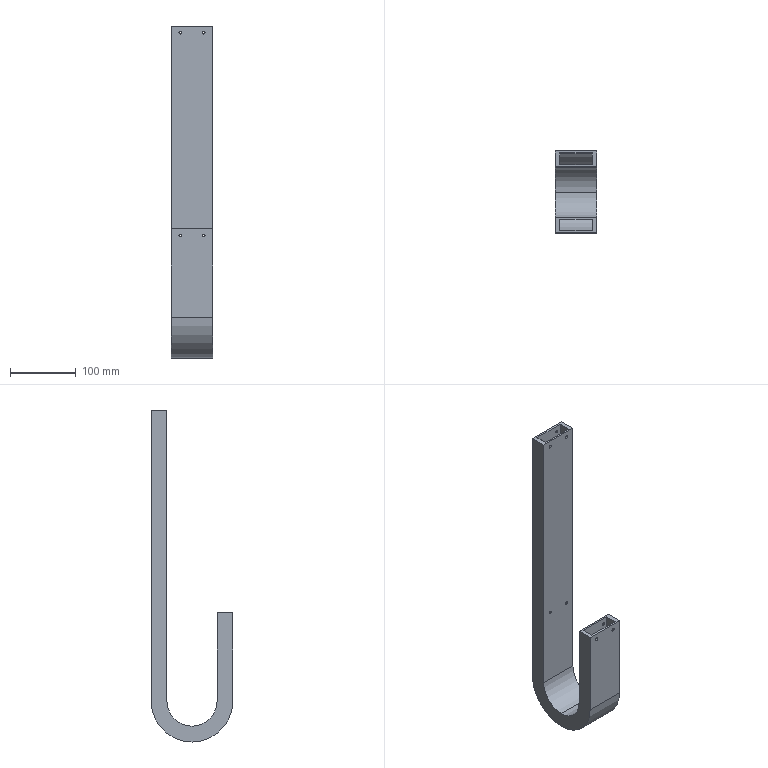Part | SolidWorks | features ICE 1, Sweep 1 | 1 solid | 46 faces | box 63 x 124 x 504 mm | volume 448072 mm3 | cylinder 32 | plane 14 | commonest cylinder face diameters 4.5 x24 76 x2 82 x2 118 x2 124 x2
STEP:
#1=CARTESIAN_POINT('',(15.25,112.,298.));
#2=VERTEX_POINT('',#1);
#3=CARTESIAN_POINT('',(19.75,112.,298.));
#4=VERTEX_POINT('',#3);
#5=CARTESIAN_POINT('',(17.5,112.,298.));
#6=DIRECTION('',(0.,-1.,0.));
#7=DIRECTION('',(1.,0.,0.));
#8=AXIS2_PLACEMENT_3D('',#5,#6,#7);
#9=CIRCLE('',#8,2.25);
#10=EDGE_CURVE('',#2,#4,#9,.T.);
#11=ORIENTED_EDGE('',*,*,#10,.F.);
#12=CARTESIAN_POINT('',(15.25,109.,298.));
#13=VERTEX_POINT('',#12);
#14=CARTESIAN_POINT('',(15.25,112.,298.));
#15=DIRECTION('',(0.,-1.,0.));
#16=VECTOR('',#15,1000.);
#17=LINE('',#14,#16);
#18=EDGE_CURVE('',#2,#13,#17,.T.);
#19=ORIENTED_EDGE('',*,*,#18,.T.);
#20=CARTESIAN_POINT('',(19.75,109.,298.));
#21=VERTEX_POINT('',#20);
#22=CARTESIAN_POINT('',(17.5,109.,298.));
#23=DIRECTION('',(0.,-1.,0.));
#24=DIRECTION('',(1.,0.,0.));
#25=AXIS2_PLACEMENT_3D('',#22,#23,#24);
#26=CIRCLE('',#25,2.25);
#27=EDGE_CURVE('',#13,#21,#26,.T.);
#28=ORIENTED_EDGE('',*,*,#27,.T.);
#29=CARTESIAN_POINT('',(19.75,112.,298.));
#30=DIRECTION('',(0.,-1.,0.));
#31=VECTOR('',#30,1000.);
#32=LINE('',#29,#31);
#33=EDGE_CURVE('',#4,#21,#32,.T.);
#34=ORIENTED_EDGE('',*,*,#33,.F.);
#35=EDGE_LOOP('',(#11,#19,#28,#34));
#36=FACE_OUTER_BOUND('',#35,.T.);
#37=CARTESIAN_POINT('',(17.5,112.,298.));
#38=DIRECTION('',(0.,-1.,0.));
#39=DIRECTION('',(1.,0.,0.));
#40=AXIS2_PLACEMENT_3D('',#37,#38,#39);
#41=CYLINDRICAL_SURFACE('',#40,2.25);
#42=ADVANCED_FACE('',(#36),#41,.F.);
#43=CARTESIAN_POINT('',(19.75,91.,298.));
#44=VERTEX_POINT('',#43);
#45=CARTESIAN_POINT('',(15.25,91.,298.));
#46=VERTEX_POINT('',#45);
#47=CARTESIAN_POINT('',(17.5,91.,298.));
#48=DIRECTION('',(0.,1.,0.));
#49=DIRECTION('',(-1.,0.,0.));
#50=AXIS2_PLACEMENT_3D('',#47,#48,#49);
#51=CIRCLE('',#50,2.25);
#52=EDGE_CURVE('',#44,#46,#51,.T.);
#53=ORIENTED_EDGE('',*,*,#52,.T.);
#54=CARTESIAN_POINT('',(15.25,88.,298.));
#55=VERTEX_POINT('',#54);
#56=CARTESIAN_POINT('',(15.25,112.,298.));
#57=DIRECTION('',(0.,-1.,0.));
#58=VECTOR('',#57,1000.);
#59=LINE('',#56,#58);
#60=EDGE_CURVE('',#46,#55,#59,.T.);
#61=ORIENTED_EDGE('',*,*,#60,.T.);
#62=CARTESIAN_POINT('',(19.75,88.,298.));
#63=VERTEX_POINT('',#62);
#64=CARTESIAN_POINT('',(17.5,88.,298.));
#65=DIRECTION('',(0.,1.,0.));
#66=DIRECTION('',(-1.,0.,0.));
#67=AXIS2_PLACEMENT_3D('',#64,#65,#66);
#68=CIRCLE('',#67,2.25);
#69=EDGE_CURVE('',#63,#55,#68,.T.);
#70=ORIENTED_EDGE('',*,*,#69,.F.);
#71=CARTESIAN_POINT('',(19.75,112.,298.));
#72=DIRECTION('',(0.,-1.,0.));
#73=VECTOR('',#72,1000.);
#74=LINE('',#71,#73);
#75=EDGE_CURVE('',#44,#63,#74,.T.);
#76=ORIENTED_EDGE('',*,*,#75,.F.);
#77=EDGE_LOOP('',(#53,#61,#70,#76));
#78=FACE_OUTER_BOUND('',#77,.T.);
#79=CARTESIAN_POINT('',(17.5,112.,298.));
#80=DIRECTION('',(0.,-1.,0.));
#81=DIRECTION('',(1.,0.,0.));
#82=AXIS2_PLACEMENT_3D('',#79,#80,#81);
#83=CYLINDRICAL_SURFACE('',#82,2.25);
#84=ADVANCED_FACE('',(#78),#83,.F.);
#85=CARTESIAN_POINT('',(-19.75,112.,298.));
#86=VERTEX_POINT('',#85);
#87=CARTESIAN_POINT('',(-15.25,112.,298.));
#88=VERTEX_POINT('',#87);
#89=CARTESIAN_POINT('',(-17.5,112.,298.));
#90=DIRECTION('',(0.,-1.,0.));
#91=DIRECTION('',(1.,0.,0.));
#92=AXIS2_PLACEMENT_3D('',#89,#90,#91);
#93=CIRCLE('',#92,2.25);
#94=EDGE_CURVE('',#86,#88,#93,.T.);
#95=ORIENTED_EDGE('',*,*,#94,.F.);
#96=CARTESIAN_POINT('',(-19.75,109.,298.));
#97=VERTEX_POINT('',#96);
#98=CARTESIAN_POINT('',(-19.75,112.,298.));
#99=DIRECTION('',(0.,-1.,0.));
#100=VECTOR('',#99,1000.);
#101=LINE('',#98,#100);
#102=EDGE_CURVE('',#86,#97,#101,.T.);
#103=ORIENTED_EDGE('',*,*,#102,.T.);
#104=CARTESIAN_POINT('',(-15.25,109.,298.));
#105=VERTEX_POINT('',#104);
#106=CARTESIAN_POINT('',(-17.5,109.,298.));
#107=DIRECTION('',(0.,-1.,0.));
#108=DIRECTION('',(1.,0.,0.));
#109=AXIS2_PLACEMENT_3D('',#106,#107,#108);
#110=CIRCLE('',#109,2.25);
#111=EDGE_CURVE('',#97,#105,#110,.T.);
#112=ORIENTED_EDGE('',*,*,#111,.T.);
#113=CARTESIAN_POINT('',(-15.25,112.,298.));
#114=DIRECTION('',(0.,-1.,0.));
#115=VECTOR('',#114,1000.);
#116=LINE('',#113,#115);
#117=EDGE_CURVE('',#88,#105,#116,.T.);
#118=ORIENTED_EDGE('',*,*,#117,.F.);
#119=EDGE_LOOP('',(#95,#103,#112,#118));
#120=FACE_OUTER_BOUND('',#119,.T.);
#121=CARTESIAN_POINT('',(-17.5,112.,298.));
#122=DIRECTION('',(0.,-1.,0.));
#123=DIRECTION('',(1.,0.,0.));
#124=AXIS2_PLACEMENT_3D('',#121,#122,#123);
#125=CYLINDRICAL_SURFACE('',#124,2.25);
#126=ADVANCED_FACE('',(#120),#125,.F.);
#127=CARTESIAN_POINT('',(-15.25,91.,298.));
#128=VERTEX_POINT('',#127);
#129=CARTESIAN_POINT('',(-19.75,91.,298.));
#130=VERTEX_POINT('',#129);
#131=CARTESIAN_POINT('',(-17.5,91.,298.));
#132=DIRECTION('',(0.,1.,0.));
#133=DIRECTION('',(-1.,0.,0.));
#134=AXIS2_PLACEMENT_3D('',#131,#132,#133);
#135=CIRCLE('',#134,2.25);
#136=EDGE_CURVE('',#128,#130,#135,.T.);
#137=ORIENTED_EDGE('',*,*,#136,.T.);
#138=CARTESIAN_POINT('',(-19.75,88.,298.));
#139=VERTEX_POINT('',#138);
#140=CARTESIAN_POINT('',(-19.75,112.,298.));
#141=DIRECTION('',(0.,-1.,0.));
#142=VECTOR('',#141,1000.);
#143=LINE('',#140,#142);
#144=EDGE_CURVE('',#130,#139,#143,.T.);
#145=ORIENTED_EDGE('',*,*,#144,.T.);
#146=CARTESIAN_POINT('',(-15.25,88.,298.));
#147=VERTEX_POINT('',#146);
#148=CARTESIAN_POINT('',(-17.5,88.,298.));
#149=DIRECTION('',(0.,1.,0.));
#150=DIRECTION('',(-1.,0.,0.));
#151=AXIS2_PLACEMENT_3D('',#148,#149,#150);
#152=CIRCLE('',#151,2.25);
#153=EDGE_CURVE('',#147,#139,#152,.T.);
#154=ORIENTED_EDGE('',*,*,#153,.F.);
#155=CARTESIAN_POINT('',(-15.25,112.,298.));
#156=DIRECTION('',(0.,-1.,0.));
#157=VECTOR('',#156,1000.);
#158=LINE('',#155,#157);
#159=EDGE_CURVE('',#128,#147,#158,.T.);
#160=ORIENTED_EDGE('',*,*,#159,.F.);
#161=EDGE_LOOP('',(#137,#145,#154,#160));
#162=FACE_OUTER_BOUND('',#161,.T.);
#163=CARTESIAN_POINT('',(-17.5,112.,298.));
#164=DIRECTION('',(0.,-1.,0.));
#165=DIRECTION('',(1.,0.,0.));
#166=AXIS2_PLACEMENT_3D('',#163,#164,#165);
#167=CYLINDRICAL_SURFACE('',#166,2.25);
#168=ADVANCED_FACE('',(#162),#167,.F.);
#169=CARTESIAN_POINT('',(15.25,112.,-10.));
#170=VERTEX_POINT('',#169);
#171=CARTESIAN_POINT('',(19.75,112.,-10.));
#172=VERTEX_POINT('',#171);
#173=CARTESIAN_POINT('',(17.5,112.,-10.));
#174=DIRECTION('',(0.,-1.,0.));
#175=DIRECTION('',(1.,0.,0.));
#176=AXIS2_PLACEMENT_3D('',#173,#174,#175);
#177=CIRCLE('',#176,2.25);
#178=EDGE_CURVE('',#170,#172,#177,.T.);
#179=ORIENTED_EDGE('',*,*,#178,.F.);
#180=CARTESIAN_POINT('',(15.25,109.,-10.));
#181=VERTEX_POINT('',#180);
#182=CARTESIAN_POINT('',(15.25,112.,-10.));
#183=DIRECTION('',(0.,-1.,0.));
#184=VECTOR('',#183,1000.);
#185=LINE('',#182,#184);
#186=EDGE_CURVE('',#170,#181,#185,.T.);
#187=ORIENTED_EDGE('',*,*,#186,.T.);
#188=CARTESIAN_POINT('',(19.75,109.,-10.));
#189=VERTEX_POINT('',#188);
#190=CARTESIAN_POINT('',(17.5,109.,-10.));
#191=DIRECTION('',(0.,-1.,0.));
#192=DIRECTION('',(1.,0.,0.));
#193=AXIS2_PLACEMENT_3D('',#190,#191,#192);
#194=CIRCLE('',#193,2.25);
#195=EDGE_CURVE('',#181,#189,#194,.T.);
#196=ORIENTED_EDGE('',*,*,#195,.T.);
#197=CARTESIAN_POINT('',(19.75,112.,-10.));
#198=DIRECTION('',(0.,-1.,0.));
#199=VECTOR('',#198,1000.);
#200=LINE('',#197,#199);
#201=EDGE_CURVE('',#172,#189,#200,.T.);
#202=ORIENTED_EDGE('',*,*,#201,.F.);
#203=EDGE_LOOP('',(#179,#187,#196,#202));
#204=FACE_OUTER_BOUND('',#203,.T.);
#205=CARTESIAN_POINT('',(17.5,112.,-10.));
#206=DIRECTION('',(0.,-1.,0.));
#207=DIRECTION('',(1.,0.,0.));
#208=AXIS2_PLACEMENT_3D('',#205,#206,#207);
#209=CYLINDRICAL_SURFACE('',#208,2.25);
#210=ADVANCED_FACE('',(#204),#209,.F.);
#211=CARTESIAN_POINT('',(19.75,91.,-10.));
#212=VERTEX_POINT('',#211);
#213=CARTESIAN_POINT('',(15.25,91.,-10.));
#214=VERTEX_POINT('',#213);
#215=CARTESIAN_POINT('',(17.5,91.,-10.));
#216=DIRECTION('',(0.,1.,0.));
#217=DIRECTION('',(-1.,0.,0.));
#218=AXIS2_PLACEMENT_3D('',#215,#216,#217);
#219=CIRCLE('',#218,2.25);
#220=EDGE_CURVE('',#212,#214,#219,.T.);
#221=ORIENTED_EDGE('',*,*,#220,.T.);
#222=CARTESIAN_POINT('',(15.25,88.,-10.));
#223=VERTEX_POINT('',#222);
#224=CARTESIAN_POINT('',(15.25,112.,-10.));
#225=DIRECTION('',(0.,-1.,0.));
#226=VECTOR('',#225,1000.);
#227=LINE('',#224,#226);
#228=EDGE_CURVE('',#214,#223,#227,.T.);
#229=ORIENTED_EDGE('',*,*,#228,.T.);
#230=CARTESIAN_POINT('',(19.75,88.,-10.));
#231=VERTEX_POINT('',#230);
#232=CARTESIAN_POINT('',(17.5,88.,-10.));
#233=DIRECTION('',(0.,1.,0.));
#234=DIRECTION('',(-1.,0.,0.));
#235=AXIS2_PLACEMENT_3D('',#232,#233,#234);
#236=CIRCLE('',#235,2.25);
#237=EDGE_CURVE('',#231,#223,#236,.T.);
#238=ORIENTED_EDGE('',*,*,#237,.F.);
#239=CARTESIAN_POINT('',(19.75,112.,-10.));
#240=DIRECTION('',(0.,-1.,0.));
#241=VECTOR('',#240,1000.);
#242=LINE('',#239,#241);
#243=EDGE_CURVE('',#212,#231,#242,.T.);
#244=ORIENTED_EDGE('',*,*,#243,.F.);
#245=EDGE_LOOP('',(#221,#229,#238,#244));
#246=FACE_OUTER_BOUND('',#245,.T.);
#247=CARTESIAN_POINT('',(17.5,112.,-10.));
#248=DIRECTION('',(0.,-1.,0.));
#249=DIRECTION('',(1.,0.,0.));
#250=AXIS2_PLACEMENT_3D('',#247,#248,#249);
#251=CYLINDRICAL_SURFACE('',#250,2.25);
#252=ADVANCED_FACE('',(#246),#251,.F.);
#253=CARTESIAN_POINT('',(19.75,12.,-10.));
#254=VERTEX_POINT('',#253);
#255=CARTESIAN_POINT('',(15.25,12.,-10.));
#256=VERTEX_POINT('',#255);
#257=CARTESIAN_POINT('',(17.5,12.,-10.));
#258=DIRECTION('',(0.,1.,0.));
#259=DIRECTION('',(-1.,0.,0.));
#260=AXIS2_PLACEMENT_3D('',#257,#258,#259);
#261=CIRCLE('',#260,2.25);
#262=EDGE_CURVE('',#254,#256,#261,.T.);
#263=ORIENTED_EDGE('',*,*,#262,.T.);
#264=CARTESIAN_POINT('',(15.25,9.,-10.));
#265=VERTEX_POINT('',#264);
#266=CARTESIAN_POINT('',(15.25,112.,-10.));
#267=DIRECTION('',(0.,-1.,0.));
#268=VECTOR('',#267,1000.);
#269=LINE('',#266,#268);
#270=EDGE_CURVE('',#256,#265,#269,.T.);
#271=ORIENTED_EDGE('',*,*,#270,.T.);
#272=CARTESIAN_POINT('',(19.75,9.,-10.));
#273=VERTEX_POINT('',#272);
#274=CARTESIAN_POINT('',(17.5,9.,-10.));
#275=DIRECTION('',(0.,1.,0.));
#276=DIRECTION('',(-1.,0.,0.));
#277=AXIS2_PLACEMENT_3D('',#274,#275,#276);
#278=CIRCLE('',#277,2.25);
#279=EDGE_CURVE('',#273,#265,#278,.T.);
#280=ORIENTED_EDGE('',*,*,#279,.F.);
#281=CARTESIAN_POINT('',(19.75,112.,-10.));
#282=DIRECTION('',(0.,-1.,0.));
#283=VECTOR('',#282,1000.);
#284=LINE('',#281,#283);
#285=EDGE_CURVE('',#254,#273,#284,.T.);
#286=ORIENTED_EDGE('',*,*,#285,.F.);
#287=EDGE_LOOP('',(#263,#271,#280,#286));
#288=FACE_OUTER_BOUND('',#287,.T.);
#289=CARTESIAN_POINT('',(17.5,112.,-10.));
#290=DIRECTION('',(0.,-1.,0.));
#291=DIRECTION('',(1.,0.,0.));
#292=AXIS2_PLACEMENT_3D('',#289,#290,#291);
#293=CYLINDRICAL_SURFACE('',#292,2.25);
#294=ADVANCED_FACE('',(#288),#293,.F.);
#295=CARTESIAN_POINT('',(15.25,-9.,-10.));
#296=VERTEX_POINT('',#295);
#297=CARTESIAN_POINT('',(19.75,-9.,-10.));
#298=VERTEX_POINT('',#297);
#299=CARTESIAN_POINT('',(17.5,-9.,-10.));
#300=DIRECTION('',(0.,-1.,0.));
#301=DIRECTION('',(1.,0.,0.));
#302=AXIS2_PLACEMENT_3D('',#299,#300,#301);
#303=CIRCLE('',#302,2.25);
#304=EDGE_CURVE('',#296,#298,#303,.T.);
#305=ORIENTED_EDGE('',*,*,#304,.F.);
#306=CARTESIAN_POINT('',(15.25,-12.,-10.));
#307=VERTEX_POINT('',#306);
#308=CARTESIAN_POINT('',(15.25,112.,-10.));
#309=DIRECTION('',(0.,-1.,0.));
#310=VECTOR('',#309,1000.);
#311=LINE('',#308,#310);
#312=EDGE_CURVE('',#296,#307,#311,.T.);
#313=ORIENTED_EDGE('',*,*,#312,.T.);
#314=CARTESIAN_POINT('',(19.75,-12.,-10.));
#315=VERTEX_POINT('',#314);
#316=CARTESIAN_POINT('',(17.5,-12.,-10.));
#317=DIRECTION('',(0.,-1.,0.));
#318=DIRECTION('',(1.,0.,0.));
#319=AXIS2_PLACEMENT_3D('',#316,#317,#318);
#320=CIRCLE('',#319,2.25);
#321=EDGE_CURVE('',#307,#315,#320,.T.);
#322=ORIENTED_EDGE('',*,*,#321,.T.);
#323=CARTESIAN_POINT('',(19.75,112.,-10.));
#324=DIRECTION('',(0.,-1.,0.));
#325=VECTOR('',#324,1000.);
#326=LINE('',#323,#325);
#327=EDGE_CURVE('',#298,#315,#326,.T.);
#328=ORIENTED_EDGE('',*,*,#327,.F.);
#329=EDGE_LOOP('',(#305,#313,#322,#328));
#330=FACE_OUTER_BOUND('',#329,.T.);
#331=CARTESIAN_POINT('',(17.5,112.,-10.));
#332=DIRECTION('',(0.,-1.,0.));
#333=DIRECTION('',(1.,0.,0.));
#334=AXIS2_PLACEMENT_3D('',#331,#332,#333);
#335=CYLINDRICAL_SURFACE('',#334,2.25);
#336=ADVANCED_FACE('',(#330),#335,.F.);
#337=CARTESIAN_POINT('',(-19.75,112.,-10.));
#338=VERTEX_POINT('',#337);
#339=CARTESIAN_POINT('',(-15.25,112.,-10.));
#340=VERTEX_POINT('',#339);
#341=CARTESIAN_POINT('',(-17.5,112.,-10.));
#342=DIRECTION('',(0.,-1.,0.));
#343=DIRECTION('',(1.,0.,0.));
#344=AXIS2_PLACEMENT_3D('',#341,#342,#343);
#345=CIRCLE('',#344,2.25);
#346=EDGE_CURVE('',#338,#340,#345,.T.);
#347=ORIENTED_EDGE('',*,*,#346,.F.);
#348=CARTESIAN_POINT('',(-19.75,109.,-10.));
#349=VERTEX_POINT('',#348);
#350=CARTESIAN_POINT('',(-19.75,112.,-10.));
#351=DIRECTION('',(0.,-1.,0.));
#352=VECTOR('',#351,1000.);
#353=LINE('',#350,#352);
#354=EDGE_CURVE('',#338,#349,#353,.T.);
#355=ORIENTED_EDGE('',*,*,#354,.T.);
#356=CARTESIAN_POINT('',(-15.25,109.,-10.));
#357=VERTEX_POINT('',#356);
#358=CARTESIAN_POINT('',(-17.5,109.,-10.));
#359=DIRECTION('',(0.,-1.,0.));
#360=DIRECTION('',(1.,0.,0.));
#361=AXIS2_PLACEMENT_3D('',#358,#359,#360);
#362=CIRCLE('',#361,2.25);
#363=EDGE_CURVE('',#349,#357,#362,.T.);
#364=ORIENTED_EDGE('',*,*,#363,.T.);
#365=CARTESIAN_POINT('',(-15.25,112.,-10.));
#366=DIRECTION('',(0.,-1.,0.));
#367=VECTOR('',#366,1000.);
#368=LINE('',#365,#367);
#369=EDGE_CURVE('',#340,#357,#368,.T.);
#370=ORIENTED_EDGE('',*,*,#369,.F.);
#371=EDGE_LOOP('',(#347,#355,#364,#370));
#372=FACE_OUTER_BOUND('',#371,.T.);
#373=CARTESIAN_POINT('',(-17.5,112.,-10.));
#374=DIRECTION('',(0.,-1.,0.));
#375=DIRECTION('',(1.,0.,0.));
#376=AXIS2_PLACEMENT_3D('',#373,#374,#375);
#377=CYLINDRICAL_SURFACE('',#376,2.25);
#378=ADVANCED_FACE('',(#372),#377,.F.);
#379=CARTESIAN_POINT('',(-15.25,91.,-10.));
#380=VERTEX_POINT('',#379);
#381=CARTESIAN_POINT('',(-19.75,91.,-10.));
#382=VERTEX_POINT('',#381);
#383=CARTESIAN_POINT('',(-17.5,91.,-10.));
#384=DIRECTION('',(0.,1.,0.));
#385=DIRECTION('',(-1.,0.,0.));
#386=AXIS2_PLACEMENT_3D('',#383,#384,#385);
#387=CIRCLE('',#386,2.25);
#388=EDGE_CURVE('',#380,#382,#387,.T.);
#389=ORIENTED_EDGE('',*,*,#388,.T.);
#390=CARTESIAN_POINT('',(-19.75,88.,-10.));
#391=VERTEX_POINT('',#390);
#392=CARTESIAN_POINT('',(-19.75,112.,-10.));
#393=DIRECTION('',(0.,-1.,0.));
#394=VECTOR('',#393,1000.);
#395=LINE('',#392,#394);
#396=EDGE_CURVE('',#382,#391,#395,.T.);
#397=ORIENTED_EDGE('',*,*,#396,.T.);
#398=CARTESIAN_POINT('',(-15.25,88.,-10.));
#399=VERTEX_POINT('',#398);
#400=CARTESIAN_POINT('',(-17.5,88.,-10.));
#401=DIRECTION('',(0.,1.,0.));
#402=DIRECTION('',(-1.,0.,0.));
#403=AXIS2_PLACEMENT_3D('',#400,#401,#402);
#404=CIRCLE('',#403,2.25);
#405=EDGE_CURVE('',#399,#391,#404,.T.);
#406=ORIENTED_EDGE('',*,*,#405,.F.);
#407=CARTESIAN_POINT('',(-15.25,112.,-10.));
#408=DIRECTION('',(0.,-1.,0.));
#409=VECTOR('',#408,1000.);
#410=LINE('',#407,#409);
#411=EDGE_CURVE('',#380,#399,#410,.T.);
#412=ORIENTED_EDGE('',*,*,#411,.F.);
#413=EDGE_LOOP('',(#389,#397,#406,#412));
#414=FACE_OUTER_BOUND('',#413,.T.);
#415=CARTESIAN_POINT('',(-17.5,112.,-10.));
#416=DIRECTION('',(0.,-1.,0.));
#417=DIRECTION('',(1.,0.,0.));
#418=AXIS2_PLACEMENT_3D('',#415,#416,#417);
#419=CYLINDRICAL_SURFACE('',#418,2.25);
#420=ADVANCED_FACE('',(#414),#419,.F.);
#421=CARTESIAN_POINT('',(-15.25,12.,-10.));
#422=VERTEX_POINT('',#421);
#423=CARTESIAN_POINT('',(-19.75,12.,-10.));
#424=VERTEX_POINT('',#423);
#425=CARTESIAN_POINT('',(-17.5,12.,-10.));
#426=DIRECTION('',(0.,1.,0.));
#427=DIRECTION('',(-1.,0.,0.));
#428=AXIS2_PLACEMENT_3D('',#425,#426,#427);
#429=CIRCLE('',#428,2.25);
#430=EDGE_CURVE('',#422,#424,#429,.T.);
#431=ORIENTED_EDGE('',*,*,#430,.T.);
#432=CARTESIAN_POINT('',(-19.75,9.,-10.));
#433=VERTEX_POINT('',#432);
#434=CARTESIAN_POINT('',(-19.75,112.,-10.));
#435=DIRECTION('',(0.,-1.,0.));
#436=VECTOR('',#435,1000.);
#437=LINE('',#434,#436);
#438=EDGE_CURVE('',#424,#433,#437,.T.);
#439=ORIENTED_EDGE('',*,*,#438,.T.);
#440=CARTESIAN_POINT('',(-15.25,9.,-10.));
#441=VERTEX_POINT('',#440);
#442=CARTESIAN_POINT('',(-17.5,9.,-10.));
#443=DIRECTION('',(0.,1.,0.));
#444=DIRECTION('',(-1.,0.,0.));
#445=AXIS2_PLACEMENT_3D('',#442,#443,#444);
#446=CIRCLE('',#445,2.25);
#447=EDGE_CURVE('',#441,#433,#446,.T.);
#448=ORIENTED_EDGE('',*,*,#447,.F.);
#449=CARTESIAN_POINT('',(-15.25,112.,-10.));
#450=DIRECTION('',(0.,-1.,0.));
#451=VECTOR('',#450,1000.);
#452=LINE('',#449,#451);
#453=EDGE_CURVE('',#422,#441,#452,.T.);
#454=ORIENTED_EDGE('',*,*,#453,.F.);
#455=EDGE_LOOP('',(#431,#439,#448,#454));
#456=FACE_OUTER_BOUND('',#455,.T.);
#457=CARTESIAN_POINT('',(-17.5,112.,-10.));
#458=DIRECTION('',(0.,-1.,0.));
#459=DIRECTION('',(1.,0.,0.));
#460=AXIS2_PLACEMENT_3D('',#457,#458,#459);
#461=CYLINDRICAL_SURFACE('',#460,2.25);
#462=ADVANCED_FACE('',(#456),#461,.F.);
#463=CARTESIAN_POINT('',(-19.75,-9.,-10.));
#464=VERTEX_POINT('',#463);
#465=CARTESIAN_POINT('',(-15.25,-9.,-10.));
#466=VERTEX_POINT('',#465);
#467=CARTESIAN_POINT('',(-17.5,-9.,-10.));
#468=DIRECTION('',(0.,-1.,0.));
#469=DIRECTION('',(1.,0.,0.));
#470=AXIS2_PLACEMENT_3D('',#467,#468,#469);
#471=CIRCLE('',#470,2.25);
#472=EDGE_CURVE('',#464,#466,#471,.T.);
#473=ORIENTED_EDGE('',*,*,#472,.F.);
#474=CARTESIAN_POINT('',(-19.75,-12.,-10.));
#475=VERTEX_POINT('',#474);
#476=CARTESIAN_POINT('',(-19.75,112.,-10.));
#477=DIRECTION('',(0.,-1.,0.));
#478=VECTOR('',#477,1000.);
#479=LINE('',#476,#478);
#480=EDGE_CURVE('',#464,#475,#479,.T.);
#481=ORIENTED_EDGE('',*,*,#480,.T.);
#482=CARTESIAN_POINT('',(-15.25,-12.,-10.));
#483=VERTEX_POINT('',#482);
#484=CARTESIAN_POINT('',(-17.5,-12.,-10.));
#485=DIRECTION('',(0.,-1.,0.));
#486=DIRECTION('',(1.,0.,0.));
#487=AXIS2_PLACEMENT_3D('',#484,#485,#486);
#488=CIRCLE('',#487,2.25);
#489=EDGE_CURVE('',#475,#483,#488,.T.);
#490=ORIENTED_EDGE('',*,*,#489,.T.);
#491=CARTESIAN_POINT('',(-15.25,112.,-10.));
#492=DIRECTION('',(0.,-1.,0.));
#493=VECTOR('',#492,1000.);
#494=LINE('',#491,#493);
#495=EDGE_CURVE('',#466,#483,#494,.T.);
#496=ORIENTED_EDGE('',*,*,#495,.F.);
#497=EDGE_LOOP('',(#473,#481,#490,#496));
#498=FACE_OUTER_BOUND('',#497,.T.);
#499=CARTESIAN_POINT('',(-17.5,112.,-10.));
#500=DIRECTION('',(0.,-1.,0.));
#501=DIRECTION('',(1.,0.,0.));
#502=AXIS2_PLACEMENT_3D('',#499,#500,#501);
#503=CYLINDRICAL_SURFACE('',#502,2.25);
#504=ADVANCED_FACE('',(#498),#503,.F.);
#505=CARTESIAN_POINT('',(-25.,9.,-134.));
#506=VERTEX_POINT('',#505);
#507=CARTESIAN_POINT('',(-25.,50.,-175.));
#508=VERTEX_POINT('',#507);
#509=CARTESIAN_POINT('',(-25.,50.,-134.));
#510=DIRECTION('',(1.,0.,0.));
#511=DIRECTION('',(0.,0.,-1.));
#512=AXIS2_PLACEMENT_3D('',#509,#510,#511);
#513=CIRCLE('',#512,41.);
#514=EDGE_CURVE('',#506,#508,#513,.T.);
#515=ORIENTED_EDGE('',*,*,#514,.T.);
#516=CARTESIAN_POINT('',(25.,50.,-175.));
#517=VERTEX_POINT('',#516);
#518=CARTESIAN_POINT('',(0.,50.,-175.));
#519=DIRECTION('',(1.,0.,0.));
#520=VECTOR('',#519,1000.);
#521=LINE('',#518,#520);
#522=EDGE_CURVE('',#508,#517,#521,.T.);
#523=ORIENTED_EDGE('',*,*,#522,.T.);
#524=CARTESIAN_POINT('',(25.,9.,-134.));
#525=VERTEX_POINT('',#524);
#526=CARTESIAN_POINT('',(25.,50.,-134.));
#527=DIRECTION('',(1.,0.,0.));
#528=DIRECTION('',(0.,0.,-1.));
#529=AXIS2_PLACEMENT_3D('',#526,#527,#528);
#530=CIRCLE('',#529,41.);
#531=EDGE_CURVE('',#525,#517,#530,.T.);
#532=ORIENTED_EDGE('',*,*,#531,.F.);
#533=CARTESIAN_POINT('',(25.,9.,-134.));
#534=DIRECTION('',(-1.,0.,0.));
#535=VECTOR('',#534,1000.);
#536=LINE('',#533,#535);
#537=EDGE_CURVE('',#525,#506,#536,.T.);
#538=ORIENTED_EDGE('',*,*,#537,.T.);
#539=EDGE_LOOP('',(#515,#523,#532,#538));
#540=FACE_OUTER_BOUND('',#539,.T.);
#541=CARTESIAN_POINT('',(0.,50.,-134.));
#542=DIRECTION('',(1.,0.,0.));
#543=DIRECTION('',(0.,0.,-1.));
#544=AXIS2_PLACEMENT_3D('',#541,#542,#543);
#545=CYLINDRICAL_SURFACE('',#544,41.);
#546=ADVANCED_FACE('',(#540),#545,.T.);
#547=CARTESIAN_POINT('',(-25.,50.,-193.));
#548=VERTEX_POINT('',#547);
#549=CARTESIAN_POINT('',(-25.,109.,-134.));
#550=VERTEX_POINT('',#549);
#551=CARTESIAN_POINT('',(-25.,50.,-134.));
#552=DIRECTION('',(1.,0.,0.));
#553=DIRECTION('',(0.,0.,-1.));
#554=AXIS2_PLACEMENT_3D('',#551,#552,#553);
#555=CIRCLE('',#554,59.);
#556=EDGE_CURVE('',#548,#550,#555,.T.);
#557=ORIENTED_EDGE('',*,*,#556,.F.);
#558=CARTESIAN_POINT('',(25.,50.,-193.));
#559=VERTEX_POINT('',#558);
#560=CARTESIAN_POINT('',(0.,50.,-193.));
#561=DIRECTION('',(1.,0.,0.));
#562=VECTOR('',#561,1000.);
#563=LINE('',#560,#562);
#564=EDGE_CURVE('',#548,#559,#563,.T.);
#565=ORIENTED_EDGE('',*,*,#564,.T.);
#566=CARTESIAN_POINT('',(25.,109.,-134.));
#567=VERTEX_POINT('',#566);
#568=CARTESIAN_POINT('',(25.,50.,-134.));
#569=DIRECTION('',(1.,0.,0.));
#570=DIRECTION('',(0.,0.,-1.));
#571=AXIS2_PLACEMENT_3D('',#568,#569,#570);
#572=CIRCLE('',#571,59.);
#573=EDGE_CURVE('',#559,#567,#572,.T.);
#574=ORIENTED_EDGE('',*,*,#573,.T.);
#575=CARTESIAN_POINT('',(25.,109.,-134.));
#576=DIRECTION('',(1.,0.,0.));
#577=VECTOR('',#576,1000.);
#578=LINE('',#575,#577);
#579=EDGE_CURVE('',#550,#567,#578,.T.);
#580=ORIENTED_EDGE('',*,*,#579,.F.);
#581=EDGE_LOOP('',(#557,#565,#574,#580));
#582=FACE_OUTER_BOUND('',#581,.T.);
#583=CARTESIAN_POINT('',(0.,50.,-134.));
#584=DIRECTION('',(1.,0.,0.));
#585=DIRECTION('',(0.,0.,-1.));
#586=AXIS2_PLACEMENT_3D('',#583,#584,#585);
#587=CYLINDRICAL_SURFACE('',#586,59.);
#588=ADVANCED_FACE('',(#582),#587,.F.);
#589=CARTESIAN_POINT('',(-31.5,-12.,-134.));
#590=VERTEX_POINT('',#589);
#591=CARTESIAN_POINT('',(-31.5,50.,-196.));
#592=VERTEX_POINT('',#591);
#593=CARTESIAN_POINT('',(-31.5,50.,-134.));
#594=DIRECTION('',(1.,0.,0.));
#595=DIRECTION('',(0.,0.,-1.));
#596=AXIS2_PLACEMENT_3D('',#593,#594,#595);
#597=CIRCLE('',#596,62.);
#598=EDGE_CURVE('',#590,#592,#597,.T.);
#599=ORIENTED_EDGE('',*,*,#598,.T.);
#600=CARTESIAN_POINT('',(31.5,50.,-196.));
#601=VERTEX_POINT('',#600);
#602=CARTESIAN_POINT('',(0.,50.,-196.));
#603=DIRECTION('',(1.,0.,0.));
#604=VECTOR('',#603,1000.);
#605=LINE('',#602,#604);
#606=EDGE_CURVE('',#592,#601,#605,.T.);
#607=ORIENTED_EDGE('',*,*,#606,.T.);
#608=CARTESIAN_POINT('',(31.5,-12.,-134.));
#609=VERTEX_POINT('',#608);
#610=CARTESIAN_POINT('',(31.5,50.,-134.));
#611=DIRECTION('',(1.,0.,0.));
#612=DIRECTION('',(0.,0.,-1.));
#613=AXIS2_PLACEMENT_3D('',#610,#611,#612);
#614=CIRCLE('',#613,62.);
#615=EDGE_CURVE('',#609,#601,#614,.T.);
#616=ORIENTED_EDGE('',*,*,#615,.F.);
#617=CARTESIAN_POINT('',(31.5,-12.,-134.));
#618=DIRECTION('',(1.,0.,0.));
#619=VECTOR('',#618,1000.);
#620=LINE('',#617,#619);
#621=EDGE_CURVE('',#590,#609,#620,.T.);
#622=ORIENTED_EDGE('',*,*,#621,.F.);
#623=EDGE_LOOP('',(#599,#607,#616,#622));
#624=FACE_OUTER_BOUND('',#623,.T.);
#625=CARTESIAN_POINT('',(0.,50.,-134.));
#626=DIRECTION('',(1.,0.,0.));
#627=DIRECTION('',(0.,0.,-1.));
#628=AXIS2_PLACEMENT_3D('',#625,#626,#627);
#629=CYLINDRICAL_SURFACE('',#628,62.);
#630=ADVANCED_FACE('',(#624),#629,.T.);
#631=CARTESIAN_POINT('',(-31.5,50.,-172.));
#632=VERTEX_POINT('',#631);
#633=CARTESIAN_POINT('',(-31.5,88.,-134.));
#634=VERTEX_POINT('',#633);
#635=CARTESIAN_POINT('',(-31.5,50.,-134.));
#636=DIRECTION('',(1.,0.,0.));
#637=DIRECTION('',(0.,0.,-1.));
#638=AXIS2_PLACEMENT_3D('',#635,#636,#637);
#639=CIRCLE('',#638,38.);
#640=EDGE_CURVE('',#632,#634,#639,.T.);
#641=ORIENTED_EDGE('',*,*,#640,.F.);
#642=CARTESIAN_POINT('',(31.5,50.,-172.));
#643=VERTEX_POINT('',#642);
#644=CARTESIAN_POINT('',(0.,50.,-172.));
#645=DIRECTION('',(1.,0.,0.));
#646=VECTOR('',#645,1000.);
#647=LINE('',#644,#646);
#648=EDGE_CURVE('',#632,#643,#647,.T.);
#649=ORIENTED_EDGE('',*,*,#648,.T.);
#650=CARTESIAN_POINT('',(31.5,88.,-134.));
#651=VERTEX_POINT('',#650);
#652=CARTESIAN_POINT('',(31.5,50.,-134.));
#653=DIRECTION('',(1.,0.,0.));
#654=DIRECTION('',(0.,0.,-1.));
#655=AXIS2_PLACEMENT_3D('',#652,#653,#654);
#656=CIRCLE('',#655,38.);
#657=EDGE_CURVE('',#643,#651,#656,.T.);
#658=ORIENTED_EDGE('',*,*,#657,.T.);
#659=CARTESIAN_POINT('',(31.5,88.,-134.));
#660=DIRECTION('',(-1.,0.,0.));
#661=VECTOR('',#660,1000.);
#662=LINE('',#659,#661);
#663=EDGE_CURVE('',#651,#634,#662,.T.);
#664=ORIENTED_EDGE('',*,*,#663,.T.);
#665=EDGE_LOOP('',(#641,#649,#658,#664));
#666=FACE_OUTER_BOUND('',#665,.T.);
#667=CARTESIAN_POINT('',(0.,50.,-134.));
#668=DIRECTION('',(1.,0.,0.));
#669=DIRECTION('',(0.,0.,-1.));
#670=AXIS2_PLACEMENT_3D('',#667,#668,#669);
#671=CYLINDRICAL_SURFACE('',#670,38.);
#672=ADVANCED_FACE('',(#666),#671,.F.);
#673=ORIENTED_EDGE('',*,*,#69,.T.);
#674=CARTESIAN_POINT('',(17.5,88.,298.));
#675=DIRECTION('',(0.,1.,0.));
#676=DIRECTION('',(-1.,0.,0.));
#677=AXIS2_PLACEMENT_3D('',#674,#675,#676);
#678=CIRCLE('',#677,2.25);
#679=EDGE_CURVE('',#55,#63,#678,.T.);
#680=ORIENTED_EDGE('',*,*,#679,.T.);
#681=EDGE_LOOP('',(#673,#680));
#682=FACE_BOUND('',#681,.T.);
#683=ORIENTED_EDGE('',*,*,#153,.T.);
#684=CARTESIAN_POINT('',(-17.5,88.,298.));
#685=DIRECTION('',(0.,1.,0.));
#686=DIRECTION('',(-1.,0.,0.));
#687=AXIS2_PLACEMENT_3D('',#684,#685,#686);
#688=CIRCLE('',#687,2.25);
#689=EDGE_CURVE('',#139,#147,#688,.T.);
#690=ORIENTED_EDGE('',*,*,#689,.T.);
#691=EDGE_LOOP('',(#683,#690));
#692=FACE_BOUND('',#691,.T.);
#693=ORIENTED_EDGE('',*,*,#237,.T.);
#694=CARTESIAN_POINT('',(17.5,88.,-10.));
#695=DIRECTION('',(0.,1.,0.));
#696=DIRECTION('',(-1.,0.,0.));
#697=AXIS2_PLACEMENT_3D('',#694,#695,#696);
#698=CIRCLE('',#697,2.25);
#699=EDGE_CURVE('',#223,#231,#698,.T.);
#700=ORIENTED_EDGE('',*,*,#699,.T.);
#701=EDGE_LOOP('',(#693,#700));
#702=FACE_BOUND('',#701,.T.);
#703=ORIENTED_EDGE('',*,*,#405,.T.);
#704=CARTESIAN_POINT('',(-17.5,88.,-10.));
#705=DIRECTION('',(0.,1.,0.));
#706=DIRECTION('',(-1.,0.,0.));
#707=AXIS2_PLACEMENT_3D('',#704,#705,#706);
#708=CIRCLE('',#707,2.25);
#709=EDGE_CURVE('',#391,#399,#708,.T.);
#710=ORIENTED_EDGE('',*,*,#709,.T.);
#711=EDGE_LOOP('',(#703,#710));
#712=FACE_BOUND('',#711,.T.);
#713=ORIENTED_EDGE('',*,*,#663,.F.);
#714=CARTESIAN_POINT('',(31.5,88.,308.));
#715=VERTEX_POINT('',#714);
#716=CARTESIAN_POINT('',(31.5,88.,-134.));
#717=DIRECTION('',(0.,0.,1.));
#718=VECTOR('',#717,1000.);
#719=LINE('',#716,#718);
#720=EDGE_CURVE('',#651,#715,#719,.T.);
#721=ORIENTED_EDGE('',*,*,#720,.T.);
#722=CARTESIAN_POINT('',(-31.5,88.,308.));
#723=VERTEX_POINT('',#722);
#724=CARTESIAN_POINT('',(31.5,88.,308.));
#725=DIRECTION('',(-1.,0.,0.));
#726=VECTOR('',#725,1000.);
#727=LINE('',#724,#726);
#728=EDGE_CURVE('',#715,#723,#727,.T.);
#729=ORIENTED_EDGE('',*,*,#728,.T.);
#730=CARTESIAN_POINT('',(-31.5,88.,-134.));
#731=DIRECTION('',(0.,0.,1.));
#732=VECTOR('',#731,1000.);
#733=LINE('',#730,#732);
#734=EDGE_CURVE('',#634,#723,#733,.T.);
#735=ORIENTED_EDGE('',*,*,#734,.F.);
#736=EDGE_LOOP('',(#713,#721,#729,#735));
#737=FACE_OUTER_BOUND('',#736,.T.);
#738=CARTESIAN_POINT('',(31.5,88.,-134.));
#739=DIRECTION('',(0.,1.,0.));
#740=DIRECTION('',(-1.,0.,0.));
#741=AXIS2_PLACEMENT_3D('',#738,#739,#740);
#742=PLANE('',#741);
#743=ADVANCED_FACE('',(#682,#692,#702,#712,#737),#742,.F.);
#744=CARTESIAN_POINT('',(17.5,112.,298.));
#745=DIRECTION('',(0.,-1.,0.));
#746=DIRECTION('',(1.,0.,0.));
#747=AXIS2_PLACEMENT_3D('',#744,#745,#746);
#748=CIRCLE('',#747,2.25);
#749=EDGE_CURVE('',#4,#2,#748,.T.);
#750=ORIENTED_EDGE('',*,*,#749,.T.);
#751=ORIENTED_EDGE('',*,*,#10,.T.);
#752=EDGE_LOOP('',(#750,#751));
#753=FACE_BOUND('',#752,.T.);
#754=CARTESIAN_POINT('',(-17.5,112.,298.));
#755=DIRECTION('',(0.,-1.,0.));
#756=DIRECTION('',(1.,0.,0.));
#757=AXIS2_PLACEMENT_3D('',#754,#755,#756);
#758=CIRCLE('',#757,2.25);
#759=EDGE_CURVE('',#88,#86,#758,.T.);
#760=ORIENTED_EDGE('',*,*,#759,.T.);
#761=ORIENTED_EDGE('',*,*,#94,.T.);
#762=EDGE_LOOP('',(#760,#761));
#763=FACE_BOUND('',#762,.T.);
#764=CARTESIAN_POINT('',(17.5,112.,-10.));
#765=DIRECTION('',(0.,-1.,0.));
#766=DIRECTION('',(1.,0.,0.));
#767=AXIS2_PLACEMENT_3D('',#764,#765,#766);
#768=CIRCLE('',#767,2.25);
#769=EDGE_CURVE('',#172,#170,#768,.T.);
#770=ORIENTED_EDGE('',*,*,#769,.T.);
#771=ORIENTED_EDGE('',*,*,#178,.T.);
#772=EDGE_LOOP('',(#770,#771));
#773=FACE_BOUND('',#772,.T.);
#774=CARTESIAN_POINT('',(-17.5,112.,-10.));
#775=DIRECTION('',(0.,-1.,0.));
#776=DIRECTION('',(1.,0.,0.));
#777=AXIS2_PLACEMENT_3D('',#774,#775,#776);
#778=CIRCLE('',#777,2.25);
#779=EDGE_CURVE('',#340,#338,#778,.T.);
#780=ORIENTED_EDGE('',*,*,#779,.T.);
#781=ORIENTED_EDGE('',*,*,#346,.T.);
#782=EDGE_LOOP('',(#780,#781));
#783=FACE_BOUND('',#782,.T.);
#784=CARTESIAN_POINT('',(-31.5,112.,-134.));
#785=VERTEX_POINT('',#784);
#786=CARTESIAN_POINT('',(31.5,112.,-134.));
#787=VERTEX_POINT('',#786);
#788=CARTESIAN_POINT('',(31.5,112.,-134.));
#789=DIRECTION('',(1.,0.,0.));
#790=VECTOR('',#789,1000.);
#791=LINE('',#788,#790);
#792=EDGE_CURVE('',#785,#787,#791,.T.);
#793=ORIENTED_EDGE('',*,*,#792,.F.);
#794=CARTESIAN_POINT('',(-31.5,112.,308.));
#795=VERTEX_POINT('',#794);
#796=CARTESIAN_POINT('',(-31.5,112.,-134.));
#797=DIRECTION('',(0.,0.,1.));
#798=VECTOR('',#797,1000.);
#799=LINE('',#796,#798);
#800=EDGE_CURVE('',#785,#795,#799,.T.);
#801=ORIENTED_EDGE('',*,*,#800,.T.);
#802=CARTESIAN_POINT('',(31.5,112.,308.));
#803=VERTEX_POINT('',#802);
#804=CARTESIAN_POINT('',(31.5,112.,308.));
#805=DIRECTION('',(1.,0.,0.));
#806=VECTOR('',#805,1000.);
#807=LINE('',#804,#806);
#808=EDGE_CURVE('',#795,#803,#807,.T.);
#809=ORIENTED_EDGE('',*,*,#808,.T.);
#810=CARTESIAN_POINT('',(31.5,112.,-134.));
#811=DIRECTION('',(0.,0.,1.));
#812=VECTOR('',#811,1000.);
#813=LINE('',#810,#812);
#814=EDGE_CURVE('',#787,#803,#813,.T.);
#815=ORIENTED_EDGE('',*,*,#814,.F.);
#816=EDGE_LOOP('',(#793,#801,#809,#815));
#817=FACE_OUTER_BOUND('',#816,.T.);
#818=CARTESIAN_POINT('',(31.5,112.,-134.));
#819=DIRECTION('',(0.,-1.,0.));
#820=DIRECTION('',(1.,0.,0.));
#821=AXIS2_PLACEMENT_3D('',#818,#819,#820);
#822=PLANE('',#821);
#823=ADVANCED_FACE('',(#753,#763,#773,#783,#817),#822,.F.);
#824=CARTESIAN_POINT('',(17.5,109.,298.));
#825=DIRECTION('',(0.,-1.,0.));
#826=DIRECTION('',(1.,0.,0.));
#827=AXIS2_PLACEMENT_3D('',#824,#825,#826);
#828=CIRCLE('',#827,2.25);
#829=EDGE_CURVE('',#21,#13,#828,.T.);
#830=ORIENTED_EDGE('',*,*,#829,.F.);
#831=ORIENTED_EDGE('',*,*,#27,.F.);
#832=EDGE_LOOP('',(#830,#831));
#833=FACE_BOUND('',#832,.T.);
#834=CARTESIAN_POINT('',(-17.5,109.,298.));
#835=DIRECTION('',(0.,-1.,0.));
#836=DIRECTION('',(1.,0.,0.));
#837=AXIS2_PLACEMENT_3D('',#834,#835,#836);
#838=CIRCLE('',#837,2.25);
#839=EDGE_CURVE('',#105,#97,#838,.T.);
#840=ORIENTED_EDGE('',*,*,#839,.F.);
#841=ORIENTED_EDGE('',*,*,#111,.F.);
#842=EDGE_LOOP('',(#840,#841));
#843=FACE_BOUND('',#842,.T.);
#844=CARTESIAN_POINT('',(17.5,109.,-10.));
#845=DIRECTION('',(0.,-1.,0.));
#846=DIRECTION('',(1.,0.,0.));
#847=AXIS2_PLACEMENT_3D('',#844,#845,#846);
#848=CIRCLE('',#847,2.25);
#849=EDGE_CURVE('',#189,#181,#848,.T.);
#850=ORIENTED_EDGE('',*,*,#849,.F.);
#851=ORIENTED_EDGE('',*,*,#195,.F.);
#852=EDGE_LOOP('',(#850,#851));
#853=FACE_BOUND('',#852,.T.);
#854=CARTESIAN_POINT('',(-17.5,109.,-10.));
#855=DIRECTION('',(0.,-1.,0.));
#856=DIRECTION('',(1.,0.,0.));
#857=AXIS2_PLACEMENT_3D('',#854,#855,#856);
#858=CIRCLE('',#857,2.25);
#859=EDGE_CURVE('',#357,#349,#858,.T.);
#860=ORIENTED_EDGE('',*,*,#859,.F.);
#861=ORIENTED_EDGE('',*,*,#363,.F.);
#862=EDGE_LOOP('',(#860,#861));
#863=FACE_BOUND('',#862,.T.);
#864=ORIENTED_EDGE('',*,*,#579,.T.);
#865=CARTESIAN_POINT('',(25.,109.,308.));
#866=VERTEX_POINT('',#865);
#867=CARTESIAN_POINT('',(25.,109.,-134.));
#868=DIRECTION('',(0.,0.,1.));
#869=VECTOR('',#868,1000.);
#870=LINE('',#867,#869);
#871=EDGE_CURVE('',#567,#866,#870,.T.);
#872=ORIENTED_EDGE('',*,*,#871,.T.);
#873=CARTESIAN_POINT('',(-25.,109.,308.));
#874=VERTEX_POINT('',#873);
#875=CARTESIAN_POINT('',(25.,109.,308.));
#876=DIRECTION('',(1.,0.,0.));
#877=VECTOR('',#876,1000.);
#878=LINE('',#875,#877);
#879=EDGE_CURVE('',#874,#866,#878,.T.);
#880=ORIENTED_EDGE('',*,*,#879,.F.);
#881=CARTESIAN_POINT('',(-25.,109.,-134.));
#882=DIRECTION('',(0.,0.,1.));
#883=VECTOR('',#882,1000.);
#884=LINE('',#881,#883);
#885=EDGE_CURVE('',#550,#874,#884,.T.);
#886=ORIENTED_EDGE('',*,*,#885,.F.);
#887=EDGE_LOOP('',(#864,#872,#880,#886));
#888=FACE_OUTER_BOUND('',#887,.T.);
#889=CARTESIAN_POINT('',(25.,109.,-134.));
#890=DIRECTION('',(0.,-1.,0.));
#891=DIRECTION('',(1.,0.,0.));
#892=AXIS2_PLACEMENT_3D('',#889,#890,#891);
#893=PLANE('',#892);
#894=ADVANCED_FACE('',(#833,#843,#853,#863,#888),#893,.T.);
#895=ORIENTED_EDGE('',*,*,#52,.F.);
#896=CARTESIAN_POINT('',(17.5,91.,298.));
#897=DIRECTION('',(0.,1.,0.));
#898=DIRECTION('',(-1.,0.,0.));
#899=AXIS2_PLACEMENT_3D('',#896,#897,#898);
#900=CIRCLE('',#899,2.25);
#901=EDGE_CURVE('',#46,#44,#900,.T.);
#902=ORIENTED_EDGE('',*,*,#901,.F.);
#903=EDGE_LOOP('',(#895,#902));
#904=FACE_BOUND('',#903,.T.);
#905=ORIENTED_EDGE('',*,*,#136,.F.);
#906=CARTESIAN_POINT('',(-17.5,91.,298.));
#907=DIRECTION('',(0.,1.,0.));
#908=DIRECTION('',(-1.,0.,0.));
#909=AXIS2_PLACEMENT_3D('',#906,#907,#908);
#910=CIRCLE('',#909,2.25);
#911=EDGE_CURVE('',#130,#128,#910,.T.);
#912=ORIENTED_EDGE('',*,*,#911,.F.);
#913=EDGE_LOOP('',(#905,#912));
#914=FACE_BOUND('',#913,.T.);
#915=ORIENTED_EDGE('',*,*,#220,.F.);
#916=CARTESIAN_POINT('',(17.5,91.,-10.));
#917=DIRECTION('',(0.,1.,0.));
#918=DIRECTION('',(-1.,0.,0.));
#919=AXIS2_PLACEMENT_3D('',#916,#917,#918);
#920=CIRCLE('',#919,2.25);
#921=EDGE_CURVE('',#214,#212,#920,.T.);
#922=ORIENTED_EDGE('',*,*,#921,.F.);
#923=EDGE_LOOP('',(#915,#922));
#924=FACE_BOUND('',#923,.T.);
#925=ORIENTED_EDGE('',*,*,#388,.F.);
#926=CARTESIAN_POINT('',(-17.5,91.,-10.));
#927=DIRECTION('',(0.,1.,0.));
#928=DIRECTION('',(-1.,0.,0.));
#929=AXIS2_PLACEMENT_3D('',#926,#927,#928);
#930=CIRCLE('',#929,2.25);
#931=EDGE_CURVE('',#382,#380,#930,.T.);
#932=ORIENTED_EDGE('',*,*,#931,.F.);
#933=EDGE_LOOP('',(#925,#932));
#934=FACE_BOUND('',#933,.T.);
#935=CARTESIAN_POINT('',(25.,91.,-134.));
#936=VERTEX_POINT('',#935);
#937=CARTESIAN_POINT('',(-25.,91.,-134.));
#938=VERTEX_POINT('',#937);
#939=CARTESIAN_POINT('',(25.,91.,-134.));
#940=DIRECTION('',(-1.,0.,0.));
#941=VECTOR('',#940,1000.);
#942=LINE('',#939,#941);
#943=EDGE_CURVE('',#936,#938,#942,.T.);
#944=ORIENTED_EDGE('',*,*,#943,.T.);
#945=CARTESIAN_POINT('',(-25.,91.,308.));
#946=VERTEX_POINT('',#945);
#947=CARTESIAN_POINT('',(-25.,91.,-134.));
#948=DIRECTION('',(0.,0.,1.));
#949=VECTOR('',#948,1000.);
#950=LINE('',#947,#949);
#951=EDGE_CURVE('',#938,#946,#950,.T.);
#952=ORIENTED_EDGE('',*,*,#951,.T.);
#953=CARTESIAN_POINT('',(25.,91.,308.));
#954=VERTEX_POINT('',#953);
#955=CARTESIAN_POINT('',(25.,91.,308.));
#956=DIRECTION('',(-1.,0.,0.));
#957=VECTOR('',#956,1000.);
#958=LINE('',#955,#957);
#959=EDGE_CURVE('',#954,#946,#958,.T.);
#960=ORIENTED_EDGE('',*,*,#959,.F.);
#961=CARTESIAN_POINT('',(25.,91.,-134.));
#962=DIRECTION('',(0.,0.,1.));
#963=VECTOR('',#962,1000.);
#964=LINE('',#961,#963);
#965=EDGE_CURVE('',#936,#954,#964,.T.);
#966=ORIENTED_EDGE('',*,*,#965,.F.);
#967=EDGE_LOOP('',(#944,#952,#960,#966));
#968=FACE_OUTER_BOUND('',#967,.T.);
#969=CARTESIAN_POINT('',(25.,91.,-134.));
#970=DIRECTION('',(0.,1.,0.));
#971=DIRECTION('',(-1.,0.,0.));
#972=AXIS2_PLACEMENT_3D('',#969,#970,#971);
#973=PLANE('',#972);
#974=ADVANCED_FACE('',(#904,#914,#924,#934,#968),#973,.T.);
#975=ORIENTED_EDGE('',*,*,#648,.F.);
#976=CARTESIAN_POINT('',(-31.5,12.,-134.));
#977=VERTEX_POINT('',#976);
#978=CARTESIAN_POINT('',(-31.5,50.,-134.));
#979=DIRECTION('',(1.,0.,0.));
#980=DIRECTION('',(0.,0.,-1.));
#981=AXIS2_PLACEMENT_3D('',#978,#979,#980);
#982=CIRCLE('',#981,38.);
#983=EDGE_CURVE('',#977,#632,#982,.T.);
#984=ORIENTED_EDGE('',*,*,#983,.F.);
#985=CARTESIAN_POINT('',(31.5,12.,-134.));
#986=VERTEX_POINT('',#985);
#987=CARTESIAN_POINT('',(31.5,12.,-134.));
#988=DIRECTION('',(-1.,0.,0.));
#989=VECTOR('',#988,1000.);
#990=LINE('',#987,#989);
#991=EDGE_CURVE('',#986,#977,#990,.T.);
#992=ORIENTED_EDGE('',*,*,#991,.F.);
#993=CARTESIAN_POINT('',(31.5,50.,-134.));
#994=DIRECTION('',(1.,0.,0.));
#995=DIRECTION('',(0.,0.,-1.));
#996=AXIS2_PLACEMENT_3D('',#993,#994,#995);
#997=CIRCLE('',#996,38.);
#998=EDGE_CURVE('',#986,#643,#997,.T.);
#999=ORIENTED_EDGE('',*,*,#998,.T.);
#1000=EDGE_LOOP('',(#975,#984,#992,#999));
#1001=FACE_OUTER_BOUND('',#1000,.T.);
#1002=CARTESIAN_POINT('',(0.,50.,-134.));
#1003=DIRECTION('',(1.,0.,0.));
#1004=DIRECTION('',(0.,0.,-1.));
#1005=AXIS2_PLACEMENT_3D('',#1002,#1003,#1004);
#1006=CYLINDRICAL_SURFACE('',#1005,38.);
#1007=ADVANCED_FACE('',(#1001),#1006,.F.);
#1008=ORIENTED_EDGE('',*,*,#606,.F.);
#1009=CARTESIAN_POINT('',(-31.5,50.,-134.));
#1010=DIRECTION('',(1.,0.,0.));
#1011=DIRECTION('',(0.,0.,-1.));
#1012=AXIS2_PLACEMENT_3D('',#1009,#1010,#1011);
#1013=CIRCLE('',#1012,62.);
#1014=EDGE_CURVE('',#592,#785,#1013,.T.);
#1015=ORIENTED_EDGE('',*,*,#1014,.T.);
#1016=ORIENTED_EDGE('',*,*,#792,.T.);
#1017=CARTESIAN_POINT('',(31.5,50.,-134.));
#1018=DIRECTION('',(1.,0.,0.));
#1019=DIRECTION('',(0.,0.,-1.));
#1020=AXIS2_PLACEMENT_3D('',#1017,#1018,#1019);
#1021=CIRCLE('',#1020,62.);
#1022=EDGE_CURVE('',#601,#787,#1021,.T.);
#1023=ORIENTED_EDGE('',*,*,#1022,.F.);
#1024=EDGE_LOOP('',(#1008,#1015,#1016,#1023));
#1025=FACE_OUTER_BOUND('',#1024,.T.);
#1026=CARTESIAN_POINT('',(0.,50.,-134.));
#1027=DIRECTION('',(1.,0.,0.));
#1028=DIRECTION('',(0.,0.,-1.));
#1029=AXIS2_PLACEMENT_3D('',#1026,#1027,#1028);
#1030=CYLINDRICAL_SURFACE('',#1029,62.);
#1031=ADVANCED_FACE('',(#1025),#1030,.T.);
#1032=ORIENTED_EDGE('',*,*,#564,.F.);
#1033=CARTESIAN_POINT('',(-25.,-9.,-134.));
#1034=VERTEX_POINT('',#1033);
#1035=CARTESIAN_POINT('',(-25.,50.,-134.));
#1036=DIRECTION('',(1.,0.,0.));
#1037=DIRECTION('',(0.,0.,-1.));
#1038=AXIS2_PLACEMENT_3D('',#1035,#1036,#1037);
#1039=CIRCLE('',#1038,59.);
#1040=EDGE_CURVE('',#1034,#548,#1039,.T.);
#1041=ORIENTED_EDGE('',*,*,#1040,.F.);
#1042=CARTESIAN_POINT('',(25.,-9.,-134.));
#1043=VERTEX_POINT('',#1042);
#1044=CARTESIAN_POINT('',(25.,-9.,-134.));
#1045=DIRECTION('',(1.,0.,0.));
#1046=VECTOR('',#1045,1000.);
#1047=LINE('',#1044,#1046);
#1048=EDGE_CURVE('',#1034,#1043,#1047,.T.);
#1049=ORIENTED_EDGE('',*,*,#1048,.T.);
#1050=CARTESIAN_POINT('',(25.,50.,-134.));
#1051=DIRECTION('',(1.,0.,0.));
#1052=DIRECTION('',(0.,0.,-1.));
#1053=AXIS2_PLACEMENT_3D('',#1050,#1051,#1052);
#1054=CIRCLE('',#1053,59.);
#1055=EDGE_CURVE('',#1043,#559,#1054,.T.);
#1056=ORIENTED_EDGE('',*,*,#1055,.T.);
#1057=EDGE_LOOP('',(#1032,#1041,#1049,#1056));
#1058=FACE_OUTER_BOUND('',#1057,.T.);
#1059=CARTESIAN_POINT('',(0.,50.,-134.));
#1060=DIRECTION('',(1.,0.,0.));
#1061=DIRECTION('',(0.,0.,-1.));
#1062=AXIS2_PLACEMENT_3D('',#1059,#1060,#1061);
#1063=CYLINDRICAL_SURFACE('',#1062,59.);
#1064=ADVANCED_FACE('',(#1058),#1063,.F.);
#1065=ORIENTED_EDGE('',*,*,#522,.F.);
#1066=CARTESIAN_POINT('',(-25.,50.,-134.));
#1067=DIRECTION('',(1.,0.,0.));
#1068=DIRECTION('',(0.,0.,-1.));
#1069=AXIS2_PLACEMENT_3D('',#1066,#1067,#1068);
#1070=CIRCLE('',#1069,41.);
#1071=EDGE_CURVE('',#508,#938,#1070,.T.);
#1072=ORIENTED_EDGE('',*,*,#1071,.T.);
#1073=ORIENTED_EDGE('',*,*,#943,.F.);
#1074=CARTESIAN_POINT('',(25.,50.,-134.));
#1075=DIRECTION('',(1.,0.,0.));
#1076=DIRECTION('',(0.,0.,-1.));
#1077=AXIS2_PLACEMENT_3D('',#1074,#1075,#1076);
#1078=CIRCLE('',#1077,41.);
#1079=EDGE_CURVE('',#517,#936,#1078,.T.);
#1080=ORIENTED_EDGE('',*,*,#1079,.F.);
#1081=EDGE_LOOP('',(#1065,#1072,#1073,#1080));
#1082=FACE_OUTER_BOUND('',#1081,.T.);
#1083=CARTESIAN_POINT('',(0.,50.,-134.));
#1084=DIRECTION('',(1.,0.,0.));
#1085=DIRECTION('',(0.,0.,-1.));
#1086=AXIS2_PLACEMENT_3D('',#1083,#1084,#1085);
#1087=CYLINDRICAL_SURFACE('',#1086,41.);
#1088=ADVANCED_FACE('',(#1082),#1087,.T.);
#1089=CARTESIAN_POINT('',(-31.5,12.,0.));
#1090=VERTEX_POINT('',#1089);
#1091=CARTESIAN_POINT('',(-31.5,-12.,0.));
#1092=VERTEX_POINT('',#1091);
#1093=CARTESIAN_POINT('',(-31.5,-12.,0.));
#1094=DIRECTION('',(0.,-1.,0.));
#1095=VECTOR('',#1094,1000.);
#1096=LINE('',#1093,#1095);
#1097=EDGE_CURVE('',#1090,#1092,#1096,.T.);
#1098=ORIENTED_EDGE('',*,*,#1097,.F.);
#1099=CARTESIAN_POINT('',(-31.5,12.,-134.));
#1100=DIRECTION('',(0.,0.,1.));
#1101=VECTOR('',#1100,1000.);
#1102=LINE('',#1099,#1101);
#1103=EDGE_CURVE('',#977,#1090,#1102,.T.);
#1104=ORIENTED_EDGE('',*,*,#1103,.F.);
#1105=ORIENTED_EDGE('',*,*,#983,.T.);
#1106=ORIENTED_EDGE('',*,*,#640,.T.);
#1107=ORIENTED_EDGE('',*,*,#734,.T.);
#1108=CARTESIAN_POINT('',(-31.5,112.,308.));
#1109=DIRECTION('',(0.,1.,0.));
#1110=VECTOR('',#1109,1000.);
#1111=LINE('',#1108,#1110);
#1112=EDGE_CURVE('',#723,#795,#1111,.T.);
#1113=ORIENTED_EDGE('',*,*,#1112,.T.);
#1114=ORIENTED_EDGE('',*,*,#800,.F.);
#1115=ORIENTED_EDGE('',*,*,#1014,.F.);
#1116=ORIENTED_EDGE('',*,*,#598,.F.);
#1117=CARTESIAN_POINT('',(-31.5,-12.,-134.));
#1118=DIRECTION('',(0.,0.,1.));
#1119=VECTOR('',#1118,1000.);
#1120=LINE('',#1117,#1119);
#1121=EDGE_CURVE('',#590,#1092,#1120,.T.);
#1122=ORIENTED_EDGE('',*,*,#1121,.T.);
#1123=EDGE_LOOP('',(#1098,#1104,#1105,#1106,#1107,#1113,#1114,#1115,#1116,#1122));
#1124=FACE_OUTER_BOUND('',#1123,.T.);
#1125=CARTESIAN_POINT('',(-31.5,-12.,-134.));
#1126=DIRECTION('',(-1.,0.,0.));
#1127=DIRECTION('',(0.,0.,1.));
#1128=AXIS2_PLACEMENT_3D('',#1125,#1126,#1127);
#1129=PLANE('',#1128);
#1130=ADVANCED_FACE('',(#1124),#1129,.T.);
#1131=ORIENTED_EDGE('',*,*,#262,.F.);
#1132=CARTESIAN_POINT('',(17.5,12.,-10.));
#1133=DIRECTION('',(0.,1.,0.));
#1134=DIRECTION('',(-1.,0.,0.));
#1135=AXIS2_PLACEMENT_3D('',#1132,#1133,#1134);
#1136=CIRCLE('',#1135,2.25);
#1137=EDGE_CURVE('',#256,#254,#1136,.T.);
#1138=ORIENTED_EDGE('',*,*,#1137,.F.);
#1139=EDGE_LOOP('',(#1131,#1138));
#1140=FACE_BOUND('',#1139,.T.);
#1141=ORIENTED_EDGE('',*,*,#430,.F.);
#1142=CARTESIAN_POINT('',(-17.5,12.,-10.));
#1143=DIRECTION('',(0.,1.,0.));
#1144=DIRECTION('',(-1.,0.,0.));
#1145=AXIS2_PLACEMENT_3D('',#1142,#1143,#1144);
#1146=CIRCLE('',#1145,2.25);
#1147=EDGE_CURVE('',#424,#422,#1146,.T.);
#1148=ORIENTED_EDGE('',*,*,#1147,.F.);
#1149=EDGE_LOOP('',(#1141,#1148));
#1150=FACE_BOUND('',#1149,.T.);
#1151=CARTESIAN_POINT('',(31.5,12.,0.));
#1152=VERTEX_POINT('',#1151);
#1153=CARTESIAN_POINT('',(31.5,12.,0.));
#1154=DIRECTION('',(-1.,0.,0.));
#1155=VECTOR('',#1154,1000.);
#1156=LINE('',#1153,#1155);
#1157=EDGE_CURVE('',#1152,#1090,#1156,.T.);
#1158=ORIENTED_EDGE('',*,*,#1157,.F.);
#1159=CARTESIAN_POINT('',(31.5,12.,-134.));
#1160=DIRECTION('',(0.,0.,1.));
#1161=VECTOR('',#1160,1000.);
#1162=LINE('',#1159,#1161);
#1163=EDGE_CURVE('',#986,#1152,#1162,.T.);
#1164=ORIENTED_EDGE('',*,*,#1163,.F.);
#1165=ORIENTED_EDGE('',*,*,#991,.T.);
#1166=ORIENTED_EDGE('',*,*,#1103,.T.);
#1167=EDGE_LOOP('',(#1158,#1164,#1165,#1166));
#1168=FACE_OUTER_BOUND('',#1167,.T.);
#1169=CARTESIAN_POINT('',(31.5,12.,-134.));
#1170=DIRECTION('',(0.,1.,0.));
#1171=DIRECTION('',(-1.,0.,0.));
#1172=AXIS2_PLACEMENT_3D('',#1169,#1170,#1171);
#1173=PLANE('',#1172);
#1174=ADVANCED_FACE('',(#1140,#1150,#1168),#1173,.T.);
#1175=CARTESIAN_POINT('',(31.5,-12.,0.));
#1176=VERTEX_POINT('',#1175);
#1177=CARTESIAN_POINT('',(31.5,-12.,0.));
#1178=DIRECTION('',(0.,1.,0.));
#1179=VECTOR('',#1178,1000.);
#1180=LINE('',#1177,#1179);
#1181=EDGE_CURVE('',#1176,#1152,#1180,.T.);
#1182=ORIENTED_EDGE('',*,*,#1181,.F.);
#1183=CARTESIAN_POINT('',(31.5,-12.,-134.));
#1184=DIRECTION('',(0.,0.,1.));
#1185=VECTOR('',#1184,1000.);
#1186=LINE('',#1183,#1185);
#1187=EDGE_CURVE('',#609,#1176,#1186,.T.);
#1188=ORIENTED_EDGE('',*,*,#1187,.F.);
#1189=ORIENTED_EDGE('',*,*,#615,.T.);
#1190=ORIENTED_EDGE('',*,*,#1022,.T.);
#1191=ORIENTED_EDGE('',*,*,#814,.T.);
#1192=CARTESIAN_POINT('',(31.5,112.,308.));
#1193=DIRECTION('',(0.,-1.,0.));
#1194=VECTOR('',#1193,1000.);
#1195=LINE('',#1192,#1194);
#1196=EDGE_CURVE('',#803,#715,#1195,.T.);
#1197=ORIENTED_EDGE('',*,*,#1196,.T.);
#1198=ORIENTED_EDGE('',*,*,#720,.F.);
#1199=ORIENTED_EDGE('',*,*,#657,.F.);
#1200=ORIENTED_EDGE('',*,*,#998,.F.);
#1201=ORIENTED_EDGE('',*,*,#1163,.T.);
#1202=EDGE_LOOP('',(#1182,#1188,#1189,#1190,#1191,#1197,#1198,#1199,#1200,#1201));
#1203=FACE_OUTER_BOUND('',#1202,.T.);
#1204=CARTESIAN_POINT('',(31.5,-12.,-134.));
#1205=DIRECTION('',(1.,0.,0.));
#1206=DIRECTION('',(0.,0.,-1.));
#1207=AXIS2_PLACEMENT_3D('',#1204,#1205,#1206);
#1208=PLANE('',#1207);
#1209=ADVANCED_FACE('',(#1203),#1208,.T.);
#1210=CARTESIAN_POINT('',(-25.,9.,0.));
#1211=VERTEX_POINT('',#1210);
#1212=CARTESIAN_POINT('',(-25.,-9.,0.));
#1213=VERTEX_POINT('',#1212);
#1214=CARTESIAN_POINT('',(-25.,-9.,0.));
#1215=DIRECTION('',(0.,-1.,0.));
#1216=VECTOR('',#1215,1000.);
#1217=LINE('',#1214,#1216);
#1218=EDGE_CURVE('',#1211,#1213,#1217,.T.);
#1219=ORIENTED_EDGE('',*,*,#1218,.T.);
#1220=CARTESIAN_POINT('',(-25.,-9.,-134.));
#1221=DIRECTION('',(0.,0.,1.));
#1222=VECTOR('',#1221,1000.);
#1223=LINE('',#1220,#1222);
#1224=EDGE_CURVE('',#1034,#1213,#1223,.T.);
#1225=ORIENTED_EDGE('',*,*,#1224,.F.);
#1226=ORIENTED_EDGE('',*,*,#1040,.T.);
#1227=ORIENTED_EDGE('',*,*,#556,.T.);
#1228=ORIENTED_EDGE('',*,*,#885,.T.);
#1229=CARTESIAN_POINT('',(-25.,109.,308.));
#1230=DIRECTION('',(0.,1.,0.));
#1231=VECTOR('',#1230,1000.);
#1232=LINE('',#1229,#1231);
#1233=EDGE_CURVE('',#946,#874,#1232,.T.);
#1234=ORIENTED_EDGE('',*,*,#1233,.F.);
#1235=ORIENTED_EDGE('',*,*,#951,.F.);
#1236=ORIENTED_EDGE('',*,*,#1071,.F.);
#1237=ORIENTED_EDGE('',*,*,#514,.F.);
#1238=CARTESIAN_POINT('',(-25.,9.,-134.));
#1239=DIRECTION('',(0.,0.,1.));
#1240=VECTOR('',#1239,1000.);
#1241=LINE('',#1238,#1240);
#1242=EDGE_CURVE('',#506,#1211,#1241,.T.);
#1243=ORIENTED_EDGE('',*,*,#1242,.T.);
#1244=EDGE_LOOP('',(#1219,#1225,#1226,#1227,#1228,#1234,#1235,#1236,#1237,#1243));
#1245=FACE_OUTER_BOUND('',#1244,.T.);
#1246=CARTESIAN_POINT('',(-25.,-9.,-134.));
#1247=DIRECTION('',(-1.,0.,0.));
#1248=DIRECTION('',(0.,0.,1.));
#1249=AXIS2_PLACEMENT_3D('',#1246,#1247,#1248);
#1250=PLANE('',#1249);
#1251=ADVANCED_FACE('',(#1245),#1250,.F.);
#1252=CARTESIAN_POINT('',(17.5,-9.,-10.));
#1253=DIRECTION('',(0.,-1.,0.));
#1254=DIRECTION('',(1.,0.,0.));
#1255=AXIS2_PLACEMENT_3D('',#1252,#1253,#1254);
#1256=CIRCLE('',#1255,2.25);
#1257=EDGE_CURVE('',#298,#296,#1256,.T.);
#1258=ORIENTED_EDGE('',*,*,#1257,.T.);
#1259=ORIENTED_EDGE('',*,*,#304,.T.);
#1260=EDGE_LOOP('',(#1258,#1259));
#1261=FACE_BOUND('',#1260,.T.);
#1262=CARTESIAN_POINT('',(-17.5,-9.,-10.));
#1263=DIRECTION('',(0.,-1.,0.));
#1264=DIRECTION('',(1.,0.,0.));
#1265=AXIS2_PLACEMENT_3D('',#1262,#1263,#1264);
#1266=CIRCLE('',#1265,2.25);
#1267=EDGE_CURVE('',#466,#464,#1266,.T.);
#1268=ORIENTED_EDGE('',*,*,#1267,.T.);
#1269=ORIENTED_EDGE('',*,*,#472,.T.);
#1270=EDGE_LOOP('',(#1268,#1269));
#1271=FACE_BOUND('',#1270,.T.);
#1272=CARTESIAN_POINT('',(25.,-9.,0.));
#1273=VERTEX_POINT('',#1272);
#1274=CARTESIAN_POINT('',(25.,-9.,0.));
#1275=DIRECTION('',(1.,0.,0.));
#1276=VECTOR('',#1275,1000.);
#1277=LINE('',#1274,#1276);
#1278=EDGE_CURVE('',#1213,#1273,#1277,.T.);
#1279=ORIENTED_EDGE('',*,*,#1278,.T.);
#1280=CARTESIAN_POINT('',(25.,-9.,-134.));
#1281=DIRECTION('',(0.,0.,1.));
#1282=VECTOR('',#1281,1000.);
#1283=LINE('',#1280,#1282);
#1284=EDGE_CURVE('',#1043,#1273,#1283,.T.);
#1285=ORIENTED_EDGE('',*,*,#1284,.F.);
#1286=ORIENTED_EDGE('',*,*,#1048,.F.);
#1287=ORIENTED_EDGE('',*,*,#1224,.T.);
#1288=EDGE_LOOP('',(#1279,#1285,#1286,#1287));
#1289=FACE_OUTER_BOUND('',#1288,.T.);
#1290=CARTESIAN_POINT('',(25.,-9.,-134.));
#1291=DIRECTION('',(0.,-1.,0.));
#1292=DIRECTION('',(1.,0.,0.));
#1293=AXIS2_PLACEMENT_3D('',#1290,#1291,#1292);
#1294=PLANE('',#1293);
#1295=ADVANCED_FACE('',(#1261,#1271,#1289),#1294,.F.);
#1296=CARTESIAN_POINT('',(25.,9.,0.));
#1297=VERTEX_POINT('',#1296);
#1298=CARTESIAN_POINT('',(25.,-9.,0.));
#1299=DIRECTION('',(0.,1.,0.));
#1300=VECTOR('',#1299,1000.);
#1301=LINE('',#1298,#1300);
#1302=EDGE_CURVE('',#1273,#1297,#1301,.T.);
#1303=ORIENTED_EDGE('',*,*,#1302,.T.);
#1304=CARTESIAN_POINT('',(25.,9.,-134.));
#1305=DIRECTION('',(0.,0.,1.));
#1306=VECTOR('',#1305,1000.);
#1307=LINE('',#1304,#1306);
#1308=EDGE_CURVE('',#525,#1297,#1307,.T.);
#1309=ORIENTED_EDGE('',*,*,#1308,.F.);
#1310=ORIENTED_EDGE('',*,*,#531,.T.);
#1311=ORIENTED_EDGE('',*,*,#1079,.T.);
#1312=ORIENTED_EDGE('',*,*,#965,.T.);
#1313=CARTESIAN_POINT('',(25.,109.,308.));
#1314=DIRECTION('',(0.,-1.,0.));
#1315=VECTOR('',#1314,1000.);
#1316=LINE('',#1313,#1315);
#1317=EDGE_CURVE('',#866,#954,#1316,.T.);
#1318=ORIENTED_EDGE('',*,*,#1317,.F.);
#1319=ORIENTED_EDGE('',*,*,#871,.F.);
#1320=ORIENTED_EDGE('',*,*,#573,.F.);
#1321=ORIENTED_EDGE('',*,*,#1055,.F.);
#1322=ORIENTED_EDGE('',*,*,#1284,.T.);
#1323=EDGE_LOOP('',(#1303,#1309,#1310,#1311,#1312,#1318,#1319,#1320,#1321,#1322));
#1324=FACE_OUTER_BOUND('',#1323,.T.);
#1325=CARTESIAN_POINT('',(25.,-9.,-134.));
#1326=DIRECTION('',(1.,0.,0.));
#1327=DIRECTION('',(0.,0.,-1.));
#1328=AXIS2_PLACEMENT_3D('',#1325,#1326,#1327);
#1329=PLANE('',#1328);
#1330=ADVANCED_FACE('',(#1324),#1329,.F.);
#1331=ORIENTED_EDGE('',*,*,#279,.T.);
#1332=CARTESIAN_POINT('',(17.5,9.,-10.));
#1333=DIRECTION('',(0.,1.,0.));
#1334=DIRECTION('',(-1.,0.,0.));
#1335=AXIS2_PLACEMENT_3D('',#1332,#1333,#1334);
#1336=CIRCLE('',#1335,2.25);
#1337=EDGE_CURVE('',#265,#273,#1336,.T.);
#1338=ORIENTED_EDGE('',*,*,#1337,.T.);
#1339=EDGE_LOOP('',(#1331,#1338));
#1340=FACE_BOUND('',#1339,.T.);
#1341=ORIENTED_EDGE('',*,*,#447,.T.);
#1342=CARTESIAN_POINT('',(-17.5,9.,-10.));
#1343=DIRECTION('',(0.,1.,0.));
#1344=DIRECTION('',(-1.,0.,0.));
#1345=AXIS2_PLACEMENT_3D('',#1342,#1343,#1344);
#1346=CIRCLE('',#1345,2.25);
#1347=EDGE_CURVE('',#433,#441,#1346,.T.);
#1348=ORIENTED_EDGE('',*,*,#1347,.T.);
#1349=EDGE_LOOP('',(#1341,#1348));
#1350=FACE_BOUND('',#1349,.T.);
#1351=CARTESIAN_POINT('',(25.,9.,0.));
#1352=DIRECTION('',(-1.,0.,0.));
#1353=VECTOR('',#1352,1000.);
#1354=LINE('',#1351,#1353);
#1355=EDGE_CURVE('',#1297,#1211,#1354,.T.);
#1356=ORIENTED_EDGE('',*,*,#1355,.T.);
#1357=ORIENTED_EDGE('',*,*,#1242,.F.);
#1358=ORIENTED_EDGE('',*,*,#537,.F.);
#1359=ORIENTED_EDGE('',*,*,#1308,.T.);
#1360=EDGE_LOOP('',(#1356,#1357,#1358,#1359));
#1361=FACE_OUTER_BOUND('',#1360,.T.);
#1362=CARTESIAN_POINT('',(25.,9.,-134.));
#1363=DIRECTION('',(0.,1.,0.));
#1364=DIRECTION('',(-1.,0.,0.));
#1365=AXIS2_PLACEMENT_3D('',#1362,#1363,#1364);
#1366=PLANE('',#1365);
#1367=ADVANCED_FACE('',(#1340,#1350,#1361),#1366,.F.);
#1368=CARTESIAN_POINT('',(17.5,-12.,-10.));
#1369=DIRECTION('',(0.,-1.,0.));
#1370=DIRECTION('',(1.,0.,0.));
#1371=AXIS2_PLACEMENT_3D('',#1368,#1369,#1370);
#1372=CIRCLE('',#1371,2.25);
#1373=EDGE_CURVE('',#315,#307,#1372,.T.);
#1374=ORIENTED_EDGE('',*,*,#1373,.F.);
#1375=ORIENTED_EDGE('',*,*,#321,.F.);
#1376=EDGE_LOOP('',(#1374,#1375));
#1377=FACE_BOUND('',#1376,.T.);
#1378=CARTESIAN_POINT('',(-17.5,-12.,-10.));
#1379=DIRECTION('',(0.,-1.,0.));
#1380=DIRECTION('',(1.,0.,0.));
#1381=AXIS2_PLACEMENT_3D('',#1378,#1379,#1380);
#1382=CIRCLE('',#1381,2.25);
#1383=EDGE_CURVE('',#483,#475,#1382,.T.);
#1384=ORIENTED_EDGE('',*,*,#1383,.F.);
#1385=ORIENTED_EDGE('',*,*,#489,.F.);
#1386=EDGE_LOOP('',(#1384,#1385));
#1387=FACE_BOUND('',#1386,.T.);
#1388=CARTESIAN_POINT('',(31.5,-12.,0.));
#1389=DIRECTION('',(1.,0.,0.));
#1390=VECTOR('',#1389,1000.);
#1391=LINE('',#1388,#1390);
#1392=EDGE_CURVE('',#1092,#1176,#1391,.T.);
#1393=ORIENTED_EDGE('',*,*,#1392,.F.);
#1394=ORIENTED_EDGE('',*,*,#1121,.F.);
#1395=ORIENTED_EDGE('',*,*,#621,.T.);
#1396=ORIENTED_EDGE('',*,*,#1187,.T.);
#1397=EDGE_LOOP('',(#1393,#1394,#1395,#1396));
#1398=FACE_OUTER_BOUND('',#1397,.T.);
#1399=CARTESIAN_POINT('',(31.5,-12.,-134.));
#1400=DIRECTION('',(0.,-1.,0.));
#1401=DIRECTION('',(1.,0.,0.));
#1402=AXIS2_PLACEMENT_3D('',#1399,#1400,#1401);
#1403=PLANE('',#1402);
#1404=ADVANCED_FACE('',(#1377,#1387,#1398),#1403,.T.);
#1405=ORIENTED_EDGE('',*,*,#1233,.T.);
#1406=ORIENTED_EDGE('',*,*,#879,.T.);
#1407=ORIENTED_EDGE('',*,*,#1317,.T.);
#1408=ORIENTED_EDGE('',*,*,#959,.T.);
#1409=EDGE_LOOP('',(#1405,#1406,#1407,#1408));
#1410=FACE_BOUND('',#1409,.T.);
#1411=ORIENTED_EDGE('',*,*,#1112,.F.);
#1412=ORIENTED_EDGE('',*,*,#728,.F.);
#1413=ORIENTED_EDGE('',*,*,#1196,.F.);
#1414=ORIENTED_EDGE('',*,*,#808,.F.);
#1415=EDGE_LOOP('',(#1411,#1412,#1413,#1414));
#1416=FACE_OUTER_BOUND('',#1415,.T.);
#1417=CARTESIAN_POINT('',(0.,100.,308.));
#1418=DIRECTION('',(0.,0.,-1.));
#1419=DIRECTION('',(1.,0.,0.));
#1420=AXIS2_PLACEMENT_3D('',#1417,#1418,#1419);
#1421=PLANE('',#1420);
#1422=ADVANCED_FACE('',(#1410,#1416),#1421,.F.);
#1423=ORIENTED_EDGE('',*,*,#1218,.F.);
#1424=ORIENTED_EDGE('',*,*,#1355,.F.);
#1425=ORIENTED_EDGE('',*,*,#1302,.F.);
#1426=ORIENTED_EDGE('',*,*,#1278,.F.);
#1427=EDGE_LOOP('',(#1423,#1424,#1425,#1426));
#1428=FACE_BOUND('',#1427,.T.);
#1429=ORIENTED_EDGE('',*,*,#1097,.T.);
#1430=ORIENTED_EDGE('',*,*,#1392,.T.);
#1431=ORIENTED_EDGE('',*,*,#1181,.T.);
#1432=ORIENTED_EDGE('',*,*,#1157,.T.);
#1433=EDGE_LOOP('',(#1429,#1430,#1431,#1432));
#1434=FACE_OUTER_BOUND('',#1433,.T.);
#1435=CARTESIAN_POINT('',(0.,0.,0.));
#1436=DIRECTION('',(0.,0.,1.));
#1437=DIRECTION('',(1.,0.,0.));
#1438=AXIS2_PLACEMENT_3D('',#1435,#1436,#1437);
#1439=PLANE('',#1438);
#1440=ADVANCED_FACE('',(#1428,#1434),#1439,.T.);
#1441=ORIENTED_EDGE('',*,*,#480,.F.);
#1442=ORIENTED_EDGE('',*,*,#1267,.F.);
#1443=ORIENTED_EDGE('',*,*,#495,.T.);
#1444=ORIENTED_EDGE('',*,*,#1383,.T.);
#1445=EDGE_LOOP('',(#1441,#1442,#1443,#1444));
#1446=FACE_OUTER_BOUND('',#1445,.T.);
#1447=CARTESIAN_POINT('',(-17.5,112.,-10.));
#1448=DIRECTION('',(0.,-1.,0.));
#1449=DIRECTION('',(1.,0.,0.));
#1450=AXIS2_PLACEMENT_3D('',#1447,#1448,#1449);
#1451=CYLINDRICAL_SURFACE('',#1450,2.25);
#1452=ADVANCED_FACE('',(#1446),#1451,.F.);
#1453=ORIENTED_EDGE('',*,*,#438,.F.);
#1454=ORIENTED_EDGE('',*,*,#1147,.T.);
#1455=ORIENTED_EDGE('',*,*,#453,.T.);
#1456=ORIENTED_EDGE('',*,*,#1347,.F.);
#1457=EDGE_LOOP('',(#1453,#1454,#1455,#1456));
#1458=FACE_OUTER_BOUND('',#1457,.T.);
#1459=CARTESIAN_POINT('',(-17.5,112.,-10.));
#1460=DIRECTION('',(0.,-1.,0.));
#1461=DIRECTION('',(1.,0.,0.));
#1462=AXIS2_PLACEMENT_3D('',#1459,#1460,#1461);
#1463=CYLINDRICAL_SURFACE('',#1462,2.25);
#1464=ADVANCED_FACE('',(#1458),#1463,.F.);
#1465=ORIENTED_EDGE('',*,*,#396,.F.);
#1466=ORIENTED_EDGE('',*,*,#931,.T.);
#1467=ORIENTED_EDGE('',*,*,#411,.T.);
#1468=ORIENTED_EDGE('',*,*,#709,.F.);
#1469=EDGE_LOOP('',(#1465,#1466,#1467,#1468));
#1470=FACE_OUTER_BOUND('',#1469,.T.);
#1471=CARTESIAN_POINT('',(-17.5,112.,-10.));
#1472=DIRECTION('',(0.,-1.,0.));
#1473=DIRECTION('',(1.,0.,0.));
#1474=AXIS2_PLACEMENT_3D('',#1471,#1472,#1473);
#1475=CYLINDRICAL_SURFACE('',#1474,2.25);
#1476=ADVANCED_FACE('',(#1470),#1475,.F.);
#1477=ORIENTED_EDGE('',*,*,#354,.F.);
#1478=ORIENTED_EDGE('',*,*,#779,.F.);
#1479=ORIENTED_EDGE('',*,*,#369,.T.);
#1480=ORIENTED_EDGE('',*,*,#859,.T.);
#1481=EDGE_LOOP('',(#1477,#1478,#1479,#1480));
#1482=FACE_OUTER_BOUND('',#1481,.T.);
#1483=CARTESIAN_POINT('',(-17.5,112.,-10.));
#1484=DIRECTION('',(0.,-1.,0.));
#1485=DIRECTION('',(1.,0.,0.));
#1486=AXIS2_PLACEMENT_3D('',#1483,#1484,#1485);
#1487=CYLINDRICAL_SURFACE('',#1486,2.25);
#1488=ADVANCED_FACE('',(#1482),#1487,.F.);
#1489=ORIENTED_EDGE('',*,*,#312,.F.);
#1490=ORIENTED_EDGE('',*,*,#1257,.F.);
#1491=ORIENTED_EDGE('',*,*,#327,.T.);
#1492=ORIENTED_EDGE('',*,*,#1373,.T.);
#1493=EDGE_LOOP('',(#1489,#1490,#1491,#1492));
#1494=FACE_OUTER_BOUND('',#1493,.T.);
#1495=CARTESIAN_POINT('',(17.5,112.,-10.));
#1496=DIRECTION('',(0.,-1.,0.));
#1497=DIRECTION('',(1.,0.,0.));
#1498=AXIS2_PLACEMENT_3D('',#1495,#1496,#1497);
#1499=CYLINDRICAL_SURFACE('',#1498,2.25);
#1500=ADVANCED_FACE('',(#1494),#1499,.F.);
#1501=ORIENTED_EDGE('',*,*,#270,.F.);
#1502=ORIENTED_EDGE('',*,*,#1137,.T.);
#1503=ORIENTED_EDGE('',*,*,#285,.T.);
#1504=ORIENTED_EDGE('',*,*,#1337,.F.);
#1505=EDGE_LOOP('',(#1501,#1502,#1503,#1504));
#1506=FACE_OUTER_BOUND('',#1505,.T.);
#1507=CARTESIAN_POINT('',(17.5,112.,-10.));
#1508=DIRECTION('',(0.,-1.,0.));
#1509=DIRECTION('',(1.,0.,0.));
#1510=AXIS2_PLACEMENT_3D('',#1507,#1508,#1509);
#1511=CYLINDRICAL_SURFACE('',#1510,2.25);
#1512=ADVANCED_FACE('',(#1506),#1511,.F.);
#1513=ORIENTED_EDGE('',*,*,#228,.F.);
#1514=ORIENTED_EDGE('',*,*,#921,.T.);
#1515=ORIENTED_EDGE('',*,*,#243,.T.);
#1516=ORIENTED_EDGE('',*,*,#699,.F.);
#1517=EDGE_LOOP('',(#1513,#1514,#1515,#1516));
#1518=FACE_OUTER_BOUND('',#1517,.T.);
#1519=CARTESIAN_POINT('',(17.5,112.,-10.));
#1520=DIRECTION('',(0.,-1.,0.));
#1521=DIRECTION('',(1.,0.,0.));
#1522=AXIS2_PLACEMENT_3D('',#1519,#1520,#1521);
#1523=CYLINDRICAL_SURFACE('',#1522,2.25);
#1524=ADVANCED_FACE('',(#1518),#1523,.F.);
#1525=ORIENTED_EDGE('',*,*,#186,.F.);
#1526=ORIENTED_EDGE('',*,*,#769,.F.);
#1527=ORIENTED_EDGE('',*,*,#201,.T.);
#1528=ORIENTED_EDGE('',*,*,#849,.T.);
#1529=EDGE_LOOP('',(#1525,#1526,#1527,#1528));
#1530=FACE_OUTER_BOUND('',#1529,.T.);
#1531=CARTESIAN_POINT('',(17.5,112.,-10.));
#1532=DIRECTION('',(0.,-1.,0.));
#1533=DIRECTION('',(1.,0.,0.));
#1534=AXIS2_PLACEMENT_3D('',#1531,#1532,#1533);
#1535=CYLINDRICAL_SURFACE('',#1534,2.25);
#1536=ADVANCED_FACE('',(#1530),#1535,.F.);
#1537=ORIENTED_EDGE('',*,*,#144,.F.);
#1538=ORIENTED_EDGE('',*,*,#911,.T.);
#1539=ORIENTED_EDGE('',*,*,#159,.T.);
#1540=ORIENTED_EDGE('',*,*,#689,.F.);
#1541=EDGE_LOOP('',(#1537,#1538,#1539,#1540));
#1542=FACE_OUTER_BOUND('',#1541,.T.);
#1543=CARTESIAN_POINT('',(-17.5,112.,298.));
#1544=DIRECTION('',(0.,-1.,0.));
#1545=DIRECTION('',(1.,0.,0.));
#1546=AXIS2_PLACEMENT_3D('',#1543,#1544,#1545);
#1547=CYLINDRICAL_SURFACE('',#1546,2.25);
#1548=ADVANCED_FACE('',(#1542),#1547,.F.);
#1549=ORIENTED_EDGE('',*,*,#102,.F.);
#1550=ORIENTED_EDGE('',*,*,#759,.F.);
#1551=ORIENTED_EDGE('',*,*,#117,.T.);
#1552=ORIENTED_EDGE('',*,*,#839,.T.);
#1553=EDGE_LOOP('',(#1549,#1550,#1551,#1552));
#1554=FACE_OUTER_BOUND('',#1553,.T.);
#1555=CARTESIAN_POINT('',(-17.5,112.,298.));
#1556=DIRECTION('',(0.,-1.,0.));
#1557=DIRECTION('',(1.,0.,0.));
#1558=AXIS2_PLACEMENT_3D('',#1555,#1556,#1557);
#1559=CYLINDRICAL_SURFACE('',#1558,2.25);
#1560=ADVANCED_FACE('',(#1554),#1559,.F.);
#1561=ORIENTED_EDGE('',*,*,#60,.F.);
#1562=ORIENTED_EDGE('',*,*,#901,.T.);
#1563=ORIENTED_EDGE('',*,*,#75,.T.);
#1564=ORIENTED_EDGE('',*,*,#679,.F.);
#1565=EDGE_LOOP('',(#1561,#1562,#1563,#1564));
#1566=FACE_OUTER_BOUND('',#1565,.T.);
#1567=CARTESIAN_POINT('',(17.5,112.,298.));
#1568=DIRECTION('',(0.,-1.,0.));
#1569=DIRECTION('',(1.,0.,0.));
#1570=AXIS2_PLACEMENT_3D('',#1567,#1568,#1569);
#1571=CYLINDRICAL_SURFACE('',#1570,2.25);
#1572=ADVANCED_FACE('',(#1566),#1571,.F.);
#1573=ORIENTED_EDGE('',*,*,#18,.F.);
#1574=ORIENTED_EDGE('',*,*,#749,.F.);
#1575=ORIENTED_EDGE('',*,*,#33,.T.);
#1576=ORIENTED_EDGE('',*,*,#829,.T.);
#1577=EDGE_LOOP('',(#1573,#1574,#1575,#1576));
#1578=FACE_OUTER_BOUND('',#1577,.T.);
#1579=CARTESIAN_POINT('',(17.5,112.,298.));
#1580=DIRECTION('',(0.,-1.,0.));
#1581=DIRECTION('',(1.,0.,0.));
#1582=AXIS2_PLACEMENT_3D('',#1579,#1580,#1581);
#1583=CYLINDRICAL_SURFACE('',#1582,2.25);
#1584=ADVANCED_FACE('',(#1578),#1583,.F.);
#1585=CLOSED_SHELL('',(#42,#84,#126,#168,#210,#252,#294,#336,#378,#420,#462,#504,#546,#588,#630,#672,#743,#823,#894,#974,#1007,#1031,#1064,#1088,#1130,#1174,#1209,#1251,#1295,#1330,#1367,#1404,#1422,#1440,#1452,#1464,#1476,#1488,#1500,#1512,#1524,#1536,#1548,#1560,#1572,#1584));
#1586=MANIFOLD_SOLID_BREP('',#1585);
#1587=CARTESIAN_POINT('',(0.,0.,0.));
#1588=DIRECTION('',(0.,0.,1.));
#1589=DIRECTION('',(1.,0.,0.));
#1590=AXIS2_PLACEMENT_3D('',#1587,#1588,#1589);
#1591=(LENGTH_UNIT()NAMED_UNIT(*)SI_UNIT(.MILLI.,.METRE.));
#1592=UNCERTAINTY_MEASURE_WITH_UNIT(LENGTH_MEASURE(0.00001),#1591,'','');
#1593=(NAMED_UNIT(*)PLANE_ANGLE_UNIT()SI_UNIT($,.RADIAN.));
#1594=(NAMED_UNIT(*)SI_UNIT($,.STERADIAN.)SOLID_ANGLE_UNIT());
#1595=(GEOMETRIC_REPRESENTATION_CONTEXT(3)GLOBAL_UNCERTAINTY_ASSIGNED_CONTEXT((#1592))GLOBAL_UNIT_ASSIGNED_CONTEXT((#1591,#1593,#1594))REPRESENTATION_CONTEXT('',''));
#1596=ADVANCED_BREP_SHAPE_REPRESENTATION('',(#1586,#1590),#1595);